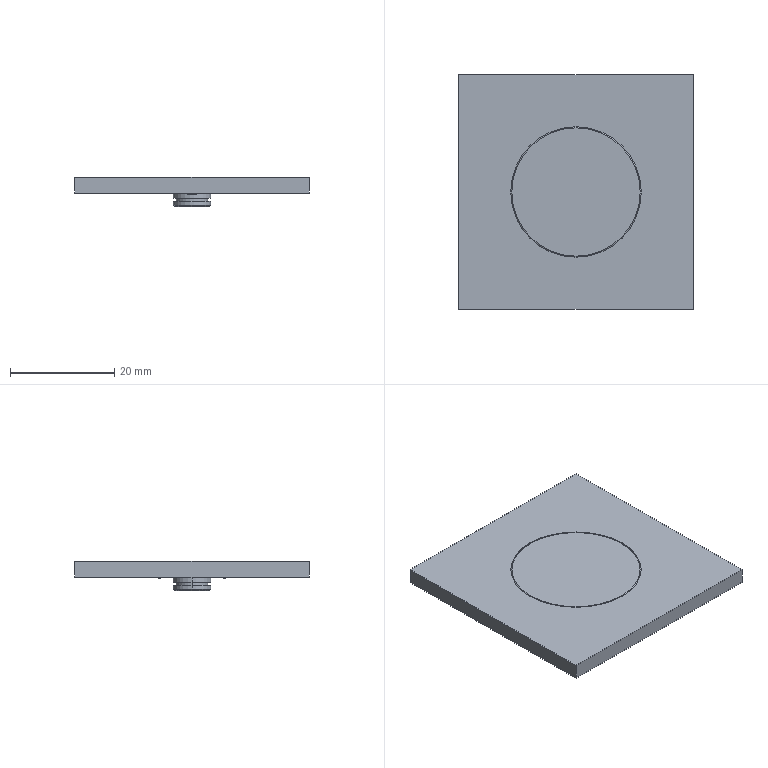Part | 2 solids | 44 faces | box 45 x 45 x 5.6 mm | volume 5766 mm3 | plane 21 | cylinder 9 | cone 8 | spline 4 | torus 2 | commonest cylinder face diameters 7.2 x4 25 x3 6 x2
STEP:
#1=CARTESIAN_POINT('',(-22.5,22.5,0.));
#2=VERTEX_POINT('',#1);
#3=CARTESIAN_POINT('',(-22.5,-22.5,0.));
#4=VERTEX_POINT('',#3);
#5=CARTESIAN_POINT('',(-22.5,22.5,0.));
#6=DIRECTION('',(0.,-1.,0.));
#7=VECTOR('',#6,1000.);
#8=LINE('',#5,#7);
#9=EDGE_CURVE('',#2,#4,#8,.T.);
#10=ORIENTED_EDGE('',*,*,#9,.F.);
#11=CARTESIAN_POINT('',(-22.5,22.5,-3.));
#12=VERTEX_POINT('',#11);
#13=CARTESIAN_POINT('',(-22.5,22.5,-3.));
#14=DIRECTION('',(0.,0.,1.));
#15=VECTOR('',#14,1000.);
#16=LINE('',#13,#15);
#17=EDGE_CURVE('',#12,#2,#16,.T.);
#18=ORIENTED_EDGE('',*,*,#17,.F.);
#19=CARTESIAN_POINT('',(-22.5,-22.5,-3.));
#20=VERTEX_POINT('',#19);
#21=CARTESIAN_POINT('',(-22.5,22.5,-3.));
#22=DIRECTION('',(0.,-1.,0.));
#23=VECTOR('',#22,1000.);
#24=LINE('',#21,#23);
#25=EDGE_CURVE('',#12,#20,#24,.T.);
#26=ORIENTED_EDGE('',*,*,#25,.T.);
#27=CARTESIAN_POINT('',(-22.5,-22.5,-3.));
#28=DIRECTION('',(0.,0.,1.));
#29=VECTOR('',#28,1000.);
#30=LINE('',#27,#29);
#31=EDGE_CURVE('',#20,#4,#30,.T.);
#32=ORIENTED_EDGE('',*,*,#31,.T.);
#33=EDGE_LOOP('',(#10,#18,#26,#32));
#34=FACE_BOUND('',#33,.T.);
#35=CARTESIAN_POINT('',(-22.5,22.5,-3.));
#36=DIRECTION('',(-1.,0.,0.));
#37=DIRECTION('',(0.,0.,1.));
#38=AXIS2_PLACEMENT_3D('',#35,#36,#37);
#39=PLANE('',#38);
#40=ADVANCED_FACE('',(#34),#39,.T.);
#41=CARTESIAN_POINT('',(22.5,-22.5,0.));
#42=VERTEX_POINT('',#41);
#43=CARTESIAN_POINT('',(-22.5,-22.5,0.));
#44=DIRECTION('',(1.,0.,0.));
#45=VECTOR('',#44,1000.);
#46=LINE('',#43,#45);
#47=EDGE_CURVE('',#4,#42,#46,.T.);
#48=ORIENTED_EDGE('',*,*,#47,.F.);
#49=ORIENTED_EDGE('',*,*,#31,.F.);
#50=CARTESIAN_POINT('',(22.5,-22.5,-3.));
#51=VERTEX_POINT('',#50);
#52=CARTESIAN_POINT('',(-22.5,-22.5,-3.));
#53=DIRECTION('',(1.,0.,0.));
#54=VECTOR('',#53,1000.);
#55=LINE('',#52,#54);
#56=EDGE_CURVE('',#20,#51,#55,.T.);
#57=ORIENTED_EDGE('',*,*,#56,.T.);
#58=CARTESIAN_POINT('',(22.5,-22.5,-3.));
#59=DIRECTION('',(0.,0.,1.));
#60=VECTOR('',#59,1000.);
#61=LINE('',#58,#60);
#62=EDGE_CURVE('',#51,#42,#61,.T.);
#63=ORIENTED_EDGE('',*,*,#62,.T.);
#64=EDGE_LOOP('',(#48,#49,#57,#63));
#65=FACE_BOUND('',#64,.T.);
#66=CARTESIAN_POINT('',(-22.5,-22.5,-3.));
#67=DIRECTION('',(0.,-1.,0.));
#68=DIRECTION('',(1.,0.,0.));
#69=AXIS2_PLACEMENT_3D('',#66,#67,#68);
#70=PLANE('',#69);
#71=ADVANCED_FACE('',(#65),#70,.T.);
#72=CARTESIAN_POINT('',(22.5,22.5,0.));
#73=VERTEX_POINT('',#72);
#74=CARTESIAN_POINT('',(22.5,-22.5,0.));
#75=DIRECTION('',(0.,1.,0.));
#76=VECTOR('',#75,1000.);
#77=LINE('',#74,#76);
#78=EDGE_CURVE('',#42,#73,#77,.T.);
#79=ORIENTED_EDGE('',*,*,#78,.F.);
#80=ORIENTED_EDGE('',*,*,#62,.F.);
#81=CARTESIAN_POINT('',(22.5,22.5,-3.));
#82=VERTEX_POINT('',#81);
#83=CARTESIAN_POINT('',(22.5,-22.5,-3.));
#84=DIRECTION('',(0.,1.,0.));
#85=VECTOR('',#84,1000.);
#86=LINE('',#83,#85);
#87=EDGE_CURVE('',#51,#82,#86,.T.);
#88=ORIENTED_EDGE('',*,*,#87,.T.);
#89=CARTESIAN_POINT('',(22.5,22.5,-3.));
#90=DIRECTION('',(0.,0.,1.));
#91=VECTOR('',#90,1000.);
#92=LINE('',#89,#91);
#93=EDGE_CURVE('',#82,#73,#92,.T.);
#94=ORIENTED_EDGE('',*,*,#93,.T.);
#95=EDGE_LOOP('',(#79,#80,#88,#94));
#96=FACE_BOUND('',#95,.T.);
#97=CARTESIAN_POINT('',(22.5,-22.5,-3.));
#98=DIRECTION('',(1.,0.,0.));
#99=DIRECTION('',(0.,1.,0.));
#100=AXIS2_PLACEMENT_3D('',#97,#98,#99);
#101=PLANE('',#100);
#102=ADVANCED_FACE('',(#96),#101,.T.);
#103=CARTESIAN_POINT('',(22.5,22.5,0.));
#104=DIRECTION('',(-1.,0.,0.));
#105=VECTOR('',#104,1000.);
#106=LINE('',#103,#105);
#107=EDGE_CURVE('',#73,#2,#106,.T.);
#108=ORIENTED_EDGE('',*,*,#107,.F.);
#109=ORIENTED_EDGE('',*,*,#93,.F.);
#110=CARTESIAN_POINT('',(22.5,22.5,-3.));
#111=DIRECTION('',(-1.,0.,0.));
#112=VECTOR('',#111,1000.);
#113=LINE('',#110,#112);
#114=EDGE_CURVE('',#82,#12,#113,.T.);
#115=ORIENTED_EDGE('',*,*,#114,.T.);
#116=ORIENTED_EDGE('',*,*,#17,.T.);
#117=EDGE_LOOP('',(#108,#109,#115,#116));
#118=FACE_BOUND('',#117,.T.);
#119=CARTESIAN_POINT('',(22.5,22.5,-3.));
#120=DIRECTION('',(0.,1.,0.));
#121=DIRECTION('',(-1.,0.,0.));
#122=AXIS2_PLACEMENT_3D('',#119,#120,#121);
#123=PLANE('',#122);
#124=ADVANCED_FACE('',(#118),#123,.T.);
#125=CARTESIAN_POINT('',(12.5,0.,-3.));
#126=VERTEX_POINT('',#125);
#127=CARTESIAN_POINT('',(0.,0.,-3.));
#128=DIRECTION('',(0.,0.,1.));
#129=DIRECTION('',(1.,0.,0.));
#130=AXIS2_PLACEMENT_3D('',#127,#128,#129);
#131=CIRCLE('',#130,12.5);
#132=EDGE_CURVE('',#126,#126,#131,.T.);
#133=ORIENTED_EDGE('',*,*,#132,.F.);
#134=EDGE_LOOP('',(#133));
#135=FACE_BOUND('',#134,.T.);
#136=CARTESIAN_POINT('',(12.5,0.,0.));
#137=VERTEX_POINT('',#136);
#138=CARTESIAN_POINT('',(0.,0.,0.));
#139=DIRECTION('',(0.,0.,1.));
#140=DIRECTION('',(1.,0.,0.));
#141=AXIS2_PLACEMENT_3D('',#138,#139,#140);
#142=CIRCLE('',#141,12.5);
#143=EDGE_CURVE('',#137,#137,#142,.T.);
#144=ORIENTED_EDGE('',*,*,#143,.T.);
#145=EDGE_LOOP('',(#144));
#146=FACE_BOUND('',#145,.T.);
#147=CARTESIAN_POINT('',(0.,0.,-3.));
#148=DIRECTION('',(0.,0.,1.));
#149=DIRECTION('',(1.,0.,0.));
#150=AXIS2_PLACEMENT_3D('',#147,#148,#149);
#151=CYLINDRICAL_SURFACE('',#150,12.5);
#152=ADVANCED_FACE('',(#135,#146),#151,.F.);
#153=ORIENTED_EDGE('',*,*,#25,.F.);
#154=ORIENTED_EDGE('',*,*,#114,.F.);
#155=ORIENTED_EDGE('',*,*,#87,.F.);
#156=ORIENTED_EDGE('',*,*,#56,.F.);
#157=EDGE_LOOP('',(#153,#154,#155,#156));
#158=FACE_BOUND('',#157,.T.);
#159=ORIENTED_EDGE('',*,*,#132,.T.);
#160=EDGE_LOOP('',(#159));
#161=FACE_BOUND('',#160,.T.);
#162=CARTESIAN_POINT('',(0.,0.,-3.));
#163=DIRECTION('',(0.,0.,1.));
#164=DIRECTION('',(1.,0.,0.));
#165=AXIS2_PLACEMENT_3D('',#162,#163,#164);
#166=PLANE('',#165);
#167=ADVANCED_FACE('',(#158,#161),#166,.F.);
#168=ORIENTED_EDGE('',*,*,#9,.T.);
#169=ORIENTED_EDGE('',*,*,#47,.T.);
#170=ORIENTED_EDGE('',*,*,#78,.T.);
#171=ORIENTED_EDGE('',*,*,#107,.T.);
#172=EDGE_LOOP('',(#168,#169,#170,#171));
#173=FACE_BOUND('',#172,.T.);
#174=ORIENTED_EDGE('',*,*,#143,.F.);
#175=EDGE_LOOP('',(#174));
#176=FACE_BOUND('',#175,.T.);
#177=CARTESIAN_POINT('',(0.,0.,0.));
#178=DIRECTION('',(0.,0.,1.));
#179=DIRECTION('',(1.,0.,0.));
#180=AXIS2_PLACEMENT_3D('',#177,#178,#179);
#181=PLANE('',#180);
#182=ADVANCED_FACE('',(#173,#176),#181,.T.);
#183=CLOSED_SHELL('',(#40,#71,#102,#124,#152,#167,#182));
#184=MANIFOLD_SOLID_BREP('',#183);
#185=CARTESIAN_POINT('',(12.2,0.,-2.1));
#186=VERTEX_POINT('',#185);
#187=CARTESIAN_POINT('',(-12.2,0.,-2.1));
#188=VERTEX_POINT('',#187);
#189=CARTESIAN_POINT('',(0.,0.,-2.1));
#190=DIRECTION('',(0.,0.,-1.));
#191=DIRECTION('',(1.,0.,0.));
#192=AXIS2_PLACEMENT_3D('',#189,#190,#191);
#193=CIRCLE('',#192,12.2);
#194=EDGE_CURVE('',#186,#188,#193,.T.);
#195=ORIENTED_EDGE('',*,*,#194,.T.);
#196=CARTESIAN_POINT('',(0.,0.,-2.1));
#197=DIRECTION('',(0.,0.,-1.));
#198=DIRECTION('',(-1.,0.,0.));
#199=AXIS2_PLACEMENT_3D('',#196,#197,#198);
#200=CIRCLE('',#199,12.2);
#201=EDGE_CURVE('',#188,#186,#200,.T.);
#202=ORIENTED_EDGE('',*,*,#201,.T.);
#203=EDGE_LOOP('',(#195,#202));
#204=FACE_BOUND('',#203,.T.);
#205=CARTESIAN_POINT('',(-0.55,6.621,-2.1));
#206=VERTEX_POINT('',#205);
#207=CARTESIAN_POINT('',(-0.55,5.779,-2.1));
#208=VERTEX_POINT('',#207);
#209=CARTESIAN_POINT('',(-0.55,6.2,-2.1));
#210=DIRECTION('',(0.,0.,1.));
#211=DIRECTION('',(0.,1.,0.));
#212=AXIS2_PLACEMENT_3D('',#209,#210,#211);
#213=CIRCLE('',#212,0.4209);
#214=EDGE_CURVE('',#206,#208,#213,.T.);
#215=ORIENTED_EDGE('',*,*,#214,.T.);
#216=CARTESIAN_POINT('',(0.55,5.779,-2.1));
#217=VERTEX_POINT('',#216);
#218=CARTESIAN_POINT('',(-0.55,5.779,-2.1));
#219=DIRECTION('',(1.,0.,0.));
#220=VECTOR('',#219,1000.);
#221=LINE('',#218,#220);
#222=EDGE_CURVE('',#208,#217,#221,.T.);
#223=ORIENTED_EDGE('',*,*,#222,.T.);
#224=CARTESIAN_POINT('',(0.55,6.621,-2.1));
#225=VERTEX_POINT('',#224);
#226=CARTESIAN_POINT('',(0.55,6.2,-2.1));
#227=DIRECTION('',(0.,0.,1.));
#228=DIRECTION('',(0.,-1.,0.));
#229=AXIS2_PLACEMENT_3D('',#226,#227,#228);
#230=CIRCLE('',#229,0.4209);
#231=EDGE_CURVE('',#217,#225,#230,.T.);
#232=ORIENTED_EDGE('',*,*,#231,.T.);
#233=CARTESIAN_POINT('',(0.55,6.621,-2.1));
#234=DIRECTION('',(-1.,0.,0.));
#235=VECTOR('',#234,1000.);
#236=LINE('',#233,#235);
#237=EDGE_CURVE('',#225,#206,#236,.T.);
#238=ORIENTED_EDGE('',*,*,#237,.T.);
#239=EDGE_LOOP('',(#215,#223,#232,#238));
#240=FACE_BOUND('',#239,.T.);
#241=CARTESIAN_POINT('',(0.55,-6.621,-2.1));
#242=VERTEX_POINT('',#241);
#243=CARTESIAN_POINT('',(0.55,-5.779,-2.1));
#244=VERTEX_POINT('',#243);
#245=CARTESIAN_POINT('',(0.55,-6.2,-2.1));
#246=DIRECTION('',(0.,0.,1.));
#247=DIRECTION('',(0.,-1.,0.));
#248=AXIS2_PLACEMENT_3D('',#245,#246,#247);
#249=CIRCLE('',#248,0.4209);
#250=EDGE_CURVE('',#242,#244,#249,.T.);
#251=ORIENTED_EDGE('',*,*,#250,.T.);
#252=CARTESIAN_POINT('',(-0.55,-5.779,-2.1));
#253=VERTEX_POINT('',#252);
#254=CARTESIAN_POINT('',(0.55,-5.779,-2.1));
#255=DIRECTION('',(-1.,0.,0.));
#256=VECTOR('',#255,1000.);
#257=LINE('',#254,#256);
#258=EDGE_CURVE('',#244,#253,#257,.T.);
#259=ORIENTED_EDGE('',*,*,#258,.T.);
#260=CARTESIAN_POINT('',(-0.55,-6.621,-2.1));
#261=VERTEX_POINT('',#260);
#262=CARTESIAN_POINT('',(-0.55,-6.2,-2.1));
#263=DIRECTION('',(0.,0.,1.));
#264=DIRECTION('',(0.,1.,0.));
#265=AXIS2_PLACEMENT_3D('',#262,#263,#264);
#266=CIRCLE('',#265,0.4209);
#267=EDGE_CURVE('',#253,#261,#266,.T.);
#268=ORIENTED_EDGE('',*,*,#267,.T.);
#269=CARTESIAN_POINT('',(-0.55,-6.621,-2.1));
#270=DIRECTION('',(1.,0.,0.));
#271=VECTOR('',#270,1000.);
#272=LINE('',#269,#271);
#273=EDGE_CURVE('',#261,#242,#272,.T.);
#274=ORIENTED_EDGE('',*,*,#273,.T.);
#275=EDGE_LOOP('',(#251,#259,#268,#274));
#276=FACE_BOUND('',#275,.T.);
#277=CARTESIAN_POINT('',(-3.6,0.,-2.1));
#278=VERTEX_POINT('',#277);
#279=CARTESIAN_POINT('',(3.6,0.,-2.1));
#280=VERTEX_POINT('',#279);
#281=CARTESIAN_POINT('',(0.,0.,-2.1));
#282=DIRECTION('',(0.,0.,1.));
#283=DIRECTION('',(-1.,0.,0.));
#284=AXIS2_PLACEMENT_3D('',#281,#282,#283);
#285=CIRCLE('',#284,3.6);
#286=EDGE_CURVE('',#278,#280,#285,.T.);
#287=ORIENTED_EDGE('',*,*,#286,.T.);
#288=CARTESIAN_POINT('',(0.,0.,-2.1));
#289=DIRECTION('',(0.,0.,1.));
#290=DIRECTION('',(1.,0.,0.));
#291=AXIS2_PLACEMENT_3D('',#288,#289,#290);
#292=CIRCLE('',#291,3.6);
#293=EDGE_CURVE('',#280,#278,#292,.T.);
#294=ORIENTED_EDGE('',*,*,#293,.T.);
#295=EDGE_LOOP('',(#287,#294));
#296=FACE_BOUND('',#295,.T.);
#297=CARTESIAN_POINT('',(0.,0.,-2.1));
#298=DIRECTION('',(0.,0.,1.));
#299=DIRECTION('',(-1.,0.,0.));
#300=AXIS2_PLACEMENT_3D('',#297,#298,#299);
#301=PLANE('',#300);
#302=ADVANCED_FACE('',(#204,#240,#276,#296),#301,.F.);
#303=CARTESIAN_POINT('',(-3.6,0.,-4.));
#304=VERTEX_POINT('',#303);
#305=CARTESIAN_POINT('',(-3.6,0.,-2.1));
#306=DIRECTION('',(0.,0.,-1.));
#307=VECTOR('',#306,1000.);
#308=LINE('',#305,#307);
#309=EDGE_CURVE('',#278,#304,#308,.T.);
#310=ORIENTED_EDGE('',*,*,#309,.F.);
#311=ORIENTED_EDGE('',*,*,#293,.F.);
#312=CARTESIAN_POINT('',(3.6,0.,-4.));
#313=VERTEX_POINT('',#312);
#314=CARTESIAN_POINT('',(3.6,0.,-2.1));
#315=DIRECTION('',(0.,0.,-1.));
#316=VECTOR('',#315,1000.);
#317=LINE('',#314,#316);
#318=EDGE_CURVE('',#280,#313,#317,.T.);
#319=ORIENTED_EDGE('',*,*,#318,.T.);
#320=CARTESIAN_POINT('',(0.,0.,-4.));
#321=DIRECTION('',(0.,0.,1.));
#322=DIRECTION('',(1.,0.,0.));
#323=AXIS2_PLACEMENT_3D('',#320,#321,#322);
#324=CIRCLE('',#323,3.6);
#325=EDGE_CURVE('',#313,#304,#324,.T.);
#326=ORIENTED_EDGE('',*,*,#325,.T.);
#327=EDGE_LOOP('',(#310,#311,#319,#326));
#328=FACE_BOUND('',#327,.T.);
#329=CARTESIAN_POINT('',(0.,0.,-2.1));
#330=DIRECTION('',(0.,0.,1.));
#331=DIRECTION('',(-1.,0.,0.));
#332=AXIS2_PLACEMENT_3D('',#329,#330,#331);
#333=CYLINDRICAL_SURFACE('',#332,3.6);
#334=ADVANCED_FACE('',(#328),#333,.T.);
#335=CARTESIAN_POINT('',(-3.6,0.,-4.6));
#336=VERTEX_POINT('',#335);
#337=CARTESIAN_POINT('',(-3.6,0.,-5.3));
#338=VERTEX_POINT('',#337);
#339=CARTESIAN_POINT('',(-3.6,0.,-4.6));
#340=DIRECTION('',(0.,-0.000000001,-1.));
#341=VECTOR('',#340,1000.);
#342=LINE('',#339,#341);
#343=EDGE_CURVE('',#336,#338,#342,.T.);
#344=ORIENTED_EDGE('',*,*,#343,.F.);
#345=CARTESIAN_POINT('',(3.6,0.,-4.6));
#346=VERTEX_POINT('',#345);
#347=CARTESIAN_POINT('',(0.,0.,-4.6));
#348=DIRECTION('',(0.,0.,1.));
#349=DIRECTION('',(1.,0.,0.));
#350=AXIS2_PLACEMENT_3D('',#347,#348,#349);
#351=CIRCLE('',#350,3.6);
#352=EDGE_CURVE('',#346,#336,#351,.T.);
#353=ORIENTED_EDGE('',*,*,#352,.F.);
#354=CARTESIAN_POINT('',(3.6,0.,-5.3));
#355=VERTEX_POINT('',#354);
#356=CARTESIAN_POINT('',(3.6,0.,-4.6));
#357=DIRECTION('',(0.,0.000000001,-1.));
#358=VECTOR('',#357,1000.);
#359=LINE('',#356,#358);
#360=EDGE_CURVE('',#346,#355,#359,.T.);
#361=ORIENTED_EDGE('',*,*,#360,.T.);
#362=CARTESIAN_POINT('',(0.,0.,-5.3));
#363=DIRECTION('',(0.,0.,-1.));
#364=DIRECTION('',(-1.,0.,0.));
#365=AXIS2_PLACEMENT_3D('',#362,#363,#364);
#366=CIRCLE('',#365,3.6);
#367=EDGE_CURVE('',#338,#355,#366,.T.);
#368=ORIENTED_EDGE('',*,*,#367,.F.);
#369=EDGE_LOOP('',(#344,#353,#361,#368));
#370=FACE_BOUND('',#369,.T.);
#371=CARTESIAN_POINT('',(0.,0.,-2.1));
#372=DIRECTION('',(0.,0.,1.));
#373=DIRECTION('',(-1.,0.,0.));
#374=AXIS2_PLACEMENT_3D('',#371,#372,#373);
#375=CYLINDRICAL_SURFACE('',#374,3.6);
#376=ADVANCED_FACE('',(#370),#375,.T.);
#377=CARTESIAN_POINT('',(0.,0.,-4.));
#378=DIRECTION('',(0.,0.,1.));
#379=DIRECTION('',(-1.,0.,0.));
#380=AXIS2_PLACEMENT_3D('',#377,#378,#379);
#381=CIRCLE('',#380,3.6);
#382=EDGE_CURVE('',#304,#313,#381,.T.);
#383=ORIENTED_EDGE('',*,*,#382,.F.);
#384=ORIENTED_EDGE('',*,*,#325,.F.);
#385=EDGE_LOOP('',(#383,#384));
#386=FACE_BOUND('',#385,.T.);
#387=CARTESIAN_POINT('',(3.,0.,-4.));
#388=VERTEX_POINT('',#387);
#389=CARTESIAN_POINT('',(-3.,0.,-4.));
#390=VERTEX_POINT('',#389);
#391=CARTESIAN_POINT('',(0.,0.,-4.));
#392=DIRECTION('',(0.,0.,1.));
#393=DIRECTION('',(1.,0.,0.));
#394=AXIS2_PLACEMENT_3D('',#391,#392,#393);
#395=CIRCLE('',#394,3.);
#396=EDGE_CURVE('',#388,#390,#395,.T.);
#397=ORIENTED_EDGE('',*,*,#396,.T.);
#398=CARTESIAN_POINT('',(0.,0.,-4.));
#399=DIRECTION('',(0.,0.,-1.));
#400=DIRECTION('',(1.,0.,0.));
#401=AXIS2_PLACEMENT_3D('',#398,#399,#400);
#402=CIRCLE('',#401,3.);
#403=EDGE_CURVE('',#388,#390,#402,.T.);
#404=ORIENTED_EDGE('',*,*,#403,.F.);
#405=EDGE_LOOP('',(#397,#404));
#406=FACE_BOUND('',#405,.T.);
#407=CARTESIAN_POINT('',(0.,0.,-4.));
#408=DIRECTION('',(0.,0.,-1.));
#409=DIRECTION('',(1.,0.,0.));
#410=AXIS2_PLACEMENT_3D('',#407,#408,#409);
#411=PLANE('',#410);
#412=ADVANCED_FACE('',(#386,#406),#411,.T.);
#413=ORIENTED_EDGE('',*,*,#403,.T.);
#414=CARTESIAN_POINT('',(-3.,0.,-4.6));
#415=VERTEX_POINT('',#414);
#416=CARTESIAN_POINT('',(-3.,0.,-4.));
#417=DIRECTION('',(0.,0.,-1.));
#418=VECTOR('',#417,1000.);
#419=LINE('',#416,#418);
#420=EDGE_CURVE('',#390,#415,#419,.T.);
#421=ORIENTED_EDGE('',*,*,#420,.T.);
#422=CARTESIAN_POINT('',(3.,0.,-4.6));
#423=VERTEX_POINT('',#422);
#424=CARTESIAN_POINT('',(0.,0.,-4.6));
#425=DIRECTION('',(0.,0.,-1.));
#426=DIRECTION('',(1.,0.,0.));
#427=AXIS2_PLACEMENT_3D('',#424,#425,#426);
#428=CIRCLE('',#427,3.);
#429=EDGE_CURVE('',#423,#415,#428,.T.);
#430=ORIENTED_EDGE('',*,*,#429,.F.);
#431=CARTESIAN_POINT('',(3.,0.,-4.));
#432=DIRECTION('',(0.,0.,-1.));
#433=VECTOR('',#432,1000.);
#434=LINE('',#431,#433);
#435=EDGE_CURVE('',#388,#423,#434,.T.);
#436=ORIENTED_EDGE('',*,*,#435,.F.);
#437=EDGE_LOOP('',(#413,#421,#430,#436));
#438=FACE_BOUND('',#437,.T.);
#439=CARTESIAN_POINT('',(0.,0.,-3.97));
#440=DIRECTION('',(0.,0.,-1.));
#441=DIRECTION('',(1.,0.,0.));
#442=AXIS2_PLACEMENT_3D('',#439,#440,#441);
#443=CYLINDRICAL_SURFACE('',#442,3.);
#444=ADVANCED_FACE('',(#438),#443,.T.);
#445=CARTESIAN_POINT('',(0.,0.,-4.6));
#446=DIRECTION('',(0.,0.,1.));
#447=DIRECTION('',(1.,0.,0.));
#448=AXIS2_PLACEMENT_3D('',#445,#446,#447);
#449=CIRCLE('',#448,3.);
#450=EDGE_CURVE('',#423,#415,#449,.T.);
#451=ORIENTED_EDGE('',*,*,#450,.T.);
#452=ORIENTED_EDGE('',*,*,#420,.F.);
#453=ORIENTED_EDGE('',*,*,#396,.F.);
#454=ORIENTED_EDGE('',*,*,#435,.T.);
#455=EDGE_LOOP('',(#451,#452,#453,#454));
#456=FACE_BOUND('',#455,.T.);
#457=CARTESIAN_POINT('',(0.,0.,-3.97));
#458=DIRECTION('',(0.,0.,-1.));
#459=DIRECTION('',(1.,0.,0.));
#460=AXIS2_PLACEMENT_3D('',#457,#458,#459);
#461=CYLINDRICAL_SURFACE('',#460,3.);
#462=ADVANCED_FACE('',(#456),#461,.T.);
#463=CARTESIAN_POINT('',(0.,0.,-4.6));
#464=DIRECTION('',(0.,0.,1.));
#465=DIRECTION('',(-1.,0.,0.));
#466=AXIS2_PLACEMENT_3D('',#463,#464,#465);
#467=CIRCLE('',#466,3.6);
#468=EDGE_CURVE('',#336,#346,#467,.T.);
#469=ORIENTED_EDGE('',*,*,#468,.T.);
#470=ORIENTED_EDGE('',*,*,#352,.T.);
#471=EDGE_LOOP('',(#469,#470));
#472=FACE_BOUND('',#471,.T.);
#473=ORIENTED_EDGE('',*,*,#429,.T.);
#474=ORIENTED_EDGE('',*,*,#450,.F.);
#475=EDGE_LOOP('',(#473,#474));
#476=FACE_BOUND('',#475,.T.);
#477=CARTESIAN_POINT('',(0.,0.,-4.6));
#478=DIRECTION('',(0.,0.,-1.));
#479=DIRECTION('',(1.,0.,0.));
#480=AXIS2_PLACEMENT_3D('',#477,#478,#479);
#481=PLANE('',#480);
#482=ADVANCED_FACE('',(#472,#476),#481,.F.);
#483=ORIENTED_EDGE('',*,*,#318,.F.);
#484=ORIENTED_EDGE('',*,*,#286,.F.);
#485=ORIENTED_EDGE('',*,*,#309,.T.);
#486=ORIENTED_EDGE('',*,*,#382,.T.);
#487=EDGE_LOOP('',(#483,#484,#485,#486));
#488=FACE_BOUND('',#487,.T.);
#489=CARTESIAN_POINT('',(0.,0.,-2.1));
#490=DIRECTION('',(0.,0.,1.));
#491=DIRECTION('',(-1.,0.,0.));
#492=AXIS2_PLACEMENT_3D('',#489,#490,#491);
#493=CYLINDRICAL_SURFACE('',#492,3.6);
#494=ADVANCED_FACE('',(#488),#493,.T.);
#495=ORIENTED_EDGE('',*,*,#360,.F.);
#496=ORIENTED_EDGE('',*,*,#468,.F.);
#497=ORIENTED_EDGE('',*,*,#343,.T.);
#498=CARTESIAN_POINT('',(0.,0.,-5.3));
#499=DIRECTION('',(0.,0.,-1.));
#500=DIRECTION('',(1.,0.,0.));
#501=AXIS2_PLACEMENT_3D('',#498,#499,#500);
#502=CIRCLE('',#501,3.6);
#503=EDGE_CURVE('',#355,#338,#502,.T.);
#504=ORIENTED_EDGE('',*,*,#503,.F.);
#505=EDGE_LOOP('',(#495,#496,#497,#504));
#506=FACE_BOUND('',#505,.T.);
#507=CARTESIAN_POINT('',(0.,0.,-2.1));
#508=DIRECTION('',(0.,0.,1.));
#509=DIRECTION('',(-1.,0.,0.));
#510=AXIS2_PLACEMENT_3D('',#507,#508,#509);
#511=CYLINDRICAL_SURFACE('',#510,3.6);
#512=ADVANCED_FACE('',(#506),#511,.T.);
#513=CARTESIAN_POINT('',(3.3,0.,-5.6));
#514=VERTEX_POINT('',#513);
#515=CARTESIAN_POINT('',(3.3,0.000000001,-5.6));
#516=DIRECTION('',(0.7071,0.,0.7071));
#517=VECTOR('',#516,1000.);
#518=LINE('',#515,#517);
#519=EDGE_CURVE('',#514,#355,#518,.T.);
#520=ORIENTED_EDGE('',*,*,#519,.T.);
#521=ORIENTED_EDGE('',*,*,#503,.T.);
#522=CARTESIAN_POINT('',(-3.3,0.,-5.6));
#523=VERTEX_POINT('',#522);
#524=CARTESIAN_POINT('',(-3.3,-0.000000001,-5.6));
#525=DIRECTION('',(-0.7071,0.,0.7071));
#526=VECTOR('',#525,1000.);
#527=LINE('',#524,#526);
#528=EDGE_CURVE('',#523,#338,#527,.T.);
#529=ORIENTED_EDGE('',*,*,#528,.F.);
#530=CARTESIAN_POINT('',(0.,0.,-5.6));
#531=DIRECTION('',(0.,0.,-1.));
#532=DIRECTION('',(1.,0.,0.));
#533=AXIS2_PLACEMENT_3D('',#530,#531,#532);
#534=CIRCLE('',#533,3.3);
#535=EDGE_CURVE('',#514,#523,#534,.T.);
#536=ORIENTED_EDGE('',*,*,#535,.F.);
#537=EDGE_LOOP('',(#520,#521,#529,#536));
#538=FACE_BOUND('',#537,.T.);
#539=CARTESIAN_POINT('',(0.,0.,-5.45));
#540=DIRECTION('',(0.,0.,1.));
#541=DIRECTION('',(0.,-1.,0.));
#542=AXIS2_PLACEMENT_3D('',#539,#540,#541);
#543=CONICAL_SURFACE('',#542,3.45,0.7854);
#544=ADVANCED_FACE('',(#538),#543,.T.);
#545=ORIENTED_EDGE('',*,*,#535,.T.);
#546=CARTESIAN_POINT('',(0.,0.,-5.6));
#547=DIRECTION('',(0.,0.,-1.));
#548=DIRECTION('',(-1.,0.,0.));
#549=AXIS2_PLACEMENT_3D('',#546,#547,#548);
#550=CIRCLE('',#549,3.3);
#551=EDGE_CURVE('',#523,#514,#550,.T.);
#552=ORIENTED_EDGE('',*,*,#551,.T.);
#553=EDGE_LOOP('',(#545,#552));
#554=FACE_BOUND('',#553,.T.);
#555=CARTESIAN_POINT('',(0.,0.,-5.6));
#556=DIRECTION('',(0.,0.,1.));
#557=DIRECTION('',(-1.,0.,0.));
#558=AXIS2_PLACEMENT_3D('',#555,#556,#557);
#559=PLANE('',#558);
#560=ADVANCED_FACE('',(#554),#559,.F.);
#561=ORIENTED_EDGE('',*,*,#528,.T.);
#562=ORIENTED_EDGE('',*,*,#367,.T.);
#563=ORIENTED_EDGE('',*,*,#519,.F.);
#564=ORIENTED_EDGE('',*,*,#551,.F.);
#565=EDGE_LOOP('',(#561,#562,#563,#564));
#566=FACE_BOUND('',#565,.T.);
#567=CARTESIAN_POINT('',(0.,0.,-5.45));
#568=DIRECTION('',(0.,0.,1.));
#569=DIRECTION('',(0.,-1.,0.));
#570=AXIS2_PLACEMENT_3D('',#567,#568,#569);
#571=CONICAL_SURFACE('',#570,3.45,0.7854);
#572=ADVANCED_FACE('',(#566),#571,.T.);
#573=CARTESIAN_POINT('',(-0.55,6.603,-3.1));
#574=VERTEX_POINT('',#573);
#575=CARTESIAN_POINT('',(-0.55,6.621,-2.1));
#576=CARTESIAN_POINT('',(-0.55,6.615,-2.433));
#577=CARTESIAN_POINT('',(-0.55,6.609,-2.767));
#578=CARTESIAN_POINT('',(-0.55,6.603,-3.1));
#579=B_SPLINE_CURVE_WITH_KNOTS('',3,(#575,#576,#577,#578),.UNSPECIFIED.,.F.,.F.,(4,4),(0.,1.),.PIECEWISE_BEZIER_KNOTS.);
#580=EDGE_CURVE('',#206,#574,#579,.T.);
#581=ORIENTED_EDGE('',*,*,#580,.F.);
#582=ORIENTED_EDGE('',*,*,#237,.F.);
#583=CARTESIAN_POINT('',(0.55,6.603,-3.1));
#584=VERTEX_POINT('',#583);
#585=CARTESIAN_POINT('',(0.55,6.603,-3.1));
#586=CARTESIAN_POINT('',(0.55,6.609,-2.767));
#587=CARTESIAN_POINT('',(0.55,6.615,-2.433));
#588=CARTESIAN_POINT('',(0.55,6.621,-2.1));
#589=B_SPLINE_CURVE_WITH_KNOTS('',3,(#585,#586,#587,#588),.UNSPECIFIED.,.F.,.F.,(4,4),(0.,1.),.PIECEWISE_BEZIER_KNOTS.);
#590=EDGE_CURVE('',#584,#225,#589,.T.);
#591=ORIENTED_EDGE('',*,*,#590,.F.);
#592=CARTESIAN_POINT('',(-0.55,6.603,-3.1));
#593=DIRECTION('',(1.,-0.000002525,0.000002569));
#594=VECTOR('',#593,1000.);
#595=LINE('',#592,#594);
#596=EDGE_CURVE('',#574,#584,#595,.T.);
#597=ORIENTED_EDGE('',*,*,#596,.F.);
#598=EDGE_LOOP('',(#581,#582,#591,#597));
#599=FACE_BOUND('',#598,.T.);
#600=CARTESIAN_POINT('',(2.31,6.6,-3.3));
#601=DIRECTION('',(0.,0.9998,-0.01745));
#602=DIRECTION('',(-1.,0.,0.));
#603=AXIS2_PLACEMENT_3D('',#600,#601,#602);
#604=PLANE('',#603);
#605=ADVANCED_FACE('',(#599),#604,.T.);
#606=CARTESIAN_POINT('',(0.55,6.4,-3.3));
#607=VERTEX_POINT('',#606);
#608=CARTESIAN_POINT('',(0.55,6.4,-3.3));
#609=DIRECTION('',(0.,0.7132,0.7009));
#610=VECTOR('',#609,1000.);
#611=LINE('',#608,#610);
#612=EDGE_CURVE('',#607,#584,#611,.T.);
#613=ORIENTED_EDGE('',*,*,#612,.F.);
#614=CARTESIAN_POINT('',(-0.55,6.4,-3.3));
#615=VERTEX_POINT('',#614);
#616=CARTESIAN_POINT('',(-0.55,6.4,-3.3));
#617=DIRECTION('',(1.,-0.000001669,0.000001698));
#618=VECTOR('',#617,1000.);
#619=LINE('',#616,#618);
#620=EDGE_CURVE('',#615,#607,#619,.T.);
#621=ORIENTED_EDGE('',*,*,#620,.F.);
#622=CARTESIAN_POINT('',(-0.55,6.4,-3.3));
#623=DIRECTION('',(-0.000000001,0.7133,0.7009));
#624=VECTOR('',#623,1000.);
#625=LINE('',#622,#624);
#626=EDGE_CURVE('',#615,#574,#625,.T.);
#627=ORIENTED_EDGE('',*,*,#626,.T.);
#628=ORIENTED_EDGE('',*,*,#596,.T.);
#629=EDGE_LOOP('',(#613,#621,#627,#628));
#630=FACE_BOUND('',#629,.T.);
#631=CARTESIAN_POINT('',(0.,6.502,-3.2));
#632=DIRECTION('',(0.,0.7009,-0.7133));
#633=DIRECTION('',(0.,-0.7133,-0.7009));
#634=AXIS2_PLACEMENT_3D('',#631,#632,#633);
#635=PLANE('',#634);
#636=ADVANCED_FACE('',(#630),#635,.T.);
#637=CARTESIAN_POINT('',(-0.55,6.,-3.3));
#638=VERTEX_POINT('',#637);
#639=CARTESIAN_POINT('',(-0.55,5.797,-3.1));
#640=VERTEX_POINT('',#639);
#641=CARTESIAN_POINT('',(-0.55,5.797,-3.1));
#642=CARTESIAN_POINT('',(-0.55,5.864,-3.167));
#643=CARTESIAN_POINT('',(-0.55,5.932,-3.233));
#644=CARTESIAN_POINT('',(-0.55,6.,-3.3));
#645=B_SPLINE_CURVE_WITH_KNOTS('',3,(#641,#642,#643,#644),.UNSPECIFIED.,.F.,.F.,(4,4),(0.,1.),.UNSPECIFIED.);
#646=EDGE_CURVE('',#638,#640,#645,.F.);
#647=ORIENTED_EDGE('',*,*,#646,.T.);
#648=CARTESIAN_POINT('',(-0.55,5.797,-3.1));
#649=CARTESIAN_POINT('',(-0.7632,5.797,-3.1));
#650=CARTESIAN_POINT('',(-1.144,6.2,-3.1));
#651=CARTESIAN_POINT('',(-0.7632,6.603,-3.1));
#652=CARTESIAN_POINT('',(-0.55,6.603,-3.1));
#653=B_SPLINE_CURVE_WITH_KNOTS('',3,(#648,#649,#650,#651,#652),.UNSPECIFIED.,.F.,.F.,(4,1,4),(0.,0.0006324,0.001265),.UNSPECIFIED.);
#654=EDGE_CURVE('',#640,#574,#653,.T.);
#655=ORIENTED_EDGE('',*,*,#654,.T.);
#656=ORIENTED_EDGE('',*,*,#626,.F.);
#657=CARTESIAN_POINT('',(-0.55,6.,-3.3));
#658=CARTESIAN_POINT('',(-0.6557,6.,-3.3));
#659=CARTESIAN_POINT('',(-0.8443,6.2,-3.3));
#660=CARTESIAN_POINT('',(-0.6557,6.4,-3.3));
#661=CARTESIAN_POINT('',(-0.55,6.4,-3.3));
#662=B_SPLINE_CURVE_WITH_KNOTS('',3,(#657,#658,#659,#660,#661),.UNSPECIFIED.,.F.,.F.,(4,1,4),(0.,0.0003126,0.0006253),.UNSPECIFIED.);
#663=EDGE_CURVE('',#638,#615,#662,.T.);
#664=ORIENTED_EDGE('',*,*,#663,.F.);
#665=EDGE_LOOP('',(#647,#655,#656,#664));
#666=FACE_BOUND('',#665,.T.);
#667=CARTESIAN_POINT('',(-0.55,6.001,-3.301));
#668=CARTESIAN_POINT('',(-0.55,5.933,-3.234));
#669=CARTESIAN_POINT('',(-0.55,5.864,-3.166));
#670=CARTESIAN_POINT('',(-0.55,5.795,-3.099));
#671=CARTESIAN_POINT('',(-0.5614,6.001,-3.301));
#672=CARTESIAN_POINT('',(-0.5654,5.933,-3.234));
#673=CARTESIAN_POINT('',(-0.5693,5.864,-3.166));
#674=CARTESIAN_POINT('',(-0.5732,5.795,-3.099));
#675=CARTESIAN_POINT('',(-0.5917,6.004,-3.301));
#676=CARTESIAN_POINT('',(-0.606,5.936,-3.234));
#677=CARTESIAN_POINT('',(-0.6204,5.868,-3.166));
#678=CARTESIAN_POINT('',(-0.6348,5.801,-3.099));
#679=CARTESIAN_POINT('',(-0.6388,6.019,-3.301));
#680=CARTESIAN_POINT('',(-0.6695,5.957,-3.234));
#681=CARTESIAN_POINT('',(-0.7002,5.894,-3.166));
#682=CARTESIAN_POINT('',(-0.7308,5.832,-3.099));
#683=CARTESIAN_POINT('',(-0.686,6.051,-3.301));
#684=CARTESIAN_POINT('',(-0.733,6.,-3.234));
#685=CARTESIAN_POINT('',(-0.78,5.949,-3.166));
#686=CARTESIAN_POINT('',(-0.8269,5.897,-3.099));
#687=CARTESIAN_POINT('',(-0.7222,6.095,-3.301));
#688=CARTESIAN_POINT('',(-0.7817,6.059,-3.234));
#689=CARTESIAN_POINT('',(-0.8412,6.023,-3.166));
#690=CARTESIAN_POINT('',(-0.9007,5.987,-3.099));
#691=CARTESIAN_POINT('',(-0.7446,6.148,-3.301));
#692=CARTESIAN_POINT('',(-0.8119,6.13,-3.234));
#693=CARTESIAN_POINT('',(-0.8791,6.112,-3.166));
#694=CARTESIAN_POINT('',(-0.9464,6.094,-3.099));
#695=CARTESIAN_POINT('',(-0.7514,6.205,-3.301));
#696=CARTESIAN_POINT('',(-0.821,6.206,-3.234));
#697=CARTESIAN_POINT('',(-0.8905,6.208,-3.166));
#698=CARTESIAN_POINT('',(-0.9601,6.21,-3.099));
#699=CARTESIAN_POINT('',(-0.742,6.261,-3.301));
#700=CARTESIAN_POINT('',(-0.8083,6.282,-3.234));
#701=CARTESIAN_POINT('',(-0.8746,6.303,-3.166));
#702=CARTESIAN_POINT('',(-0.9409,6.324,-3.099));
#703=CARTESIAN_POINT('',(-0.7171,6.313,-3.301));
#704=CARTESIAN_POINT('',(-0.7748,6.351,-3.234));
#705=CARTESIAN_POINT('',(-0.8326,6.39,-3.166));
#706=CARTESIAN_POINT('',(-0.8903,6.429,-3.099));
#707=CARTESIAN_POINT('',(-0.6788,6.355,-3.301));
#708=CARTESIAN_POINT('',(-0.7233,6.408,-3.234));
#709=CARTESIAN_POINT('',(-0.7679,6.462,-3.166));
#710=CARTESIAN_POINT('',(-0.8124,6.515,-3.099));
#711=CARTESIAN_POINT('',(-0.6301,6.385,-3.301));
#712=CARTESIAN_POINT('',(-0.6578,6.449,-3.234));
#713=CARTESIAN_POINT('',(-0.6855,6.513,-3.166));
#714=CARTESIAN_POINT('',(-0.7131,6.576,-3.099));
#715=CARTESIAN_POINT('',(-0.5855,6.397,-3.301));
#716=CARTESIAN_POINT('',(-0.5977,6.465,-3.234));
#717=CARTESIAN_POINT('',(-0.61,6.533,-3.166));
#718=CARTESIAN_POINT('',(-0.6223,6.601,-3.099));
#719=CARTESIAN_POINT('',(-0.5583,6.399,-3.301));
#720=CARTESIAN_POINT('',(-0.5612,6.467,-3.234));
#721=CARTESIAN_POINT('',(-0.5641,6.536,-3.166));
#722=CARTESIAN_POINT('',(-0.567,6.605,-3.099));
#723=CARTESIAN_POINT('',(-0.55,6.399,-3.301));
#724=CARTESIAN_POINT('',(-0.55,6.467,-3.234));
#725=CARTESIAN_POINT('',(-0.55,6.536,-3.166));
#726=CARTESIAN_POINT('',(-0.55,6.605,-3.099));
#727=B_SPLINE_SURFACE_WITH_KNOTS('',3,3,((#667,#668,#669,#670),(#671,#672,#673,#674),(#675,#676,#677,#678),(#679,#680,#681,#682),(#683,#684,#685,#686),(#687,#688,#689,#690),(#691,#692,#693,#694),(#695,#696,#697,#698),(#699,#700,#701,#702),(#703,#704,#705,#706),(#707,#708,#709,#710),(#711,#712,#713,#714),(#715,#716,#717,#718),(#719,#720,#721,#722),(#723,#724,#725,#726)),.RULED_SURF.,.F.,.F.,.F.,(4,1,1,1,1,1,1,1,1,1,1,1,4),(4,4),(0.02701,0.07885,0.1645,0.2501,0.3358,0.4214,0.507,0.5927,0.6783,0.764,0.8496,0.9353,0.9731),(0.09595,0.904),.UNSPECIFIED.);
#728=ADVANCED_FACE('',(#666),#727,.F.);
#729=CARTESIAN_POINT('',(0.55,6.,-3.3));
#730=VERTEX_POINT('',#729);
#731=CARTESIAN_POINT('',(0.55,6.,-3.3));
#732=DIRECTION('',(-1.,-0.000000541,-0.00000055));
#733=VECTOR('',#732,1000.);
#734=LINE('',#731,#733);
#735=EDGE_CURVE('',#730,#638,#734,.T.);
#736=ORIENTED_EDGE('',*,*,#735,.T.);
#737=ORIENTED_EDGE('',*,*,#663,.T.);
#738=ORIENTED_EDGE('',*,*,#620,.T.);
#739=CARTESIAN_POINT('',(0.55,6.4,-3.3));
#740=CARTESIAN_POINT('',(0.6557,6.4,-3.3));
#741=CARTESIAN_POINT('',(0.8443,6.2,-3.3));
#742=CARTESIAN_POINT('',(0.6557,6.,-3.3));
#743=CARTESIAN_POINT('',(0.55,6.,-3.3));
#744=B_SPLINE_CURVE_WITH_KNOTS('',3,(#739,#740,#741,#742,#743),.UNSPECIFIED.,.F.,.F.,(4,1,4),(0.,0.0003126,0.0006252),.UNSPECIFIED.);
#745=EDGE_CURVE('',#607,#730,#744,.T.);
#746=ORIENTED_EDGE('',*,*,#745,.T.);
#747=EDGE_LOOP('',(#736,#737,#738,#746));
#748=FACE_BOUND('',#747,.T.);
#749=CARTESIAN_POINT('',(0.,0.,-3.3));
#750=DIRECTION('',(0.,0.,1.));
#751=DIRECTION('',(-1.,0.,0.));
#752=AXIS2_PLACEMENT_3D('',#749,#750,#751);
#753=PLANE('',#752);
#754=ADVANCED_FACE('',(#748),#753,.F.);
#755=CARTESIAN_POINT('',(0.55,-6.4,-3.3));
#756=VERTEX_POINT('',#755);
#757=CARTESIAN_POINT('',(-0.55,-6.4,-3.3));
#758=VERTEX_POINT('',#757);
#759=CARTESIAN_POINT('',(0.55,-6.4,-3.3));
#760=DIRECTION('',(-1.,-0.000000541,-0.00000055));
#761=VECTOR('',#760,1000.);
#762=LINE('',#759,#761);
#763=EDGE_CURVE('',#756,#758,#762,.T.);
#764=ORIENTED_EDGE('',*,*,#763,.T.);
#765=CARTESIAN_POINT('',(-0.55,-6.,-3.3));
#766=VERTEX_POINT('',#765);
#767=CARTESIAN_POINT('',(-0.55,-6.4,-3.3));
#768=CARTESIAN_POINT('',(-0.6557,-6.4,-3.3));
#769=CARTESIAN_POINT('',(-0.8443,-6.2,-3.3));
#770=CARTESIAN_POINT('',(-0.6557,-6.,-3.3));
#771=CARTESIAN_POINT('',(-0.55,-6.,-3.3));
#772=B_SPLINE_CURVE_WITH_KNOTS('',3,(#767,#768,#769,#770,#771),.UNSPECIFIED.,.F.,.F.,(4,1,4),(0.,0.0003126,0.0006253),.UNSPECIFIED.);
#773=EDGE_CURVE('',#758,#766,#772,.T.);
#774=ORIENTED_EDGE('',*,*,#773,.T.);
#775=CARTESIAN_POINT('',(0.55,-6.,-3.3));
#776=VERTEX_POINT('',#775);
#777=CARTESIAN_POINT('',(-0.55,-6.,-3.3));
#778=DIRECTION('',(1.,-0.000001669,0.000001698));
#779=VECTOR('',#778,1000.);
#780=LINE('',#777,#779);
#781=EDGE_CURVE('',#766,#776,#780,.T.);
#782=ORIENTED_EDGE('',*,*,#781,.T.);
#783=CARTESIAN_POINT('',(0.55,-6.,-3.3));
#784=CARTESIAN_POINT('',(0.6557,-6.,-3.3));
#785=CARTESIAN_POINT('',(0.8443,-6.2,-3.3));
#786=CARTESIAN_POINT('',(0.6557,-6.4,-3.3));
#787=CARTESIAN_POINT('',(0.55,-6.4,-3.3));
#788=B_SPLINE_CURVE_WITH_KNOTS('',3,(#783,#784,#785,#786,#787),.UNSPECIFIED.,.F.,.F.,(4,1,4),(0.,0.0003126,0.0006252),.UNSPECIFIED.);
#789=EDGE_CURVE('',#776,#756,#788,.T.);
#790=ORIENTED_EDGE('',*,*,#789,.T.);
#791=EDGE_LOOP('',(#764,#774,#782,#790));
#792=FACE_BOUND('',#791,.T.);
#793=CARTESIAN_POINT('',(0.,0.,-3.3));
#794=DIRECTION('',(0.,0.,1.));
#795=DIRECTION('',(-1.,0.,0.));
#796=AXIS2_PLACEMENT_3D('',#793,#794,#795);
#797=PLANE('',#796);
#798=ADVANCED_FACE('',(#792),#797,.F.);
#799=ORIENTED_EDGE('',*,*,#612,.T.);
#800=CARTESIAN_POINT('',(0.55,5.797,-3.1));
#801=VERTEX_POINT('',#800);
#802=CARTESIAN_POINT('',(0.55,6.603,-3.1));
#803=CARTESIAN_POINT('',(0.7632,6.603,-3.1));
#804=CARTESIAN_POINT('',(1.144,6.2,-3.1));
#805=CARTESIAN_POINT('',(0.7632,5.797,-3.1));
#806=CARTESIAN_POINT('',(0.55,5.797,-3.1));
#807=B_SPLINE_CURVE_WITH_KNOTS('',3,(#802,#803,#804,#805,#806),.UNSPECIFIED.,.F.,.F.,(4,1,4),(0.000000001,0.0006319,0.001264),.UNSPECIFIED.);
#808=EDGE_CURVE('',#584,#801,#807,.T.);
#809=ORIENTED_EDGE('',*,*,#808,.T.);
#810=CARTESIAN_POINT('',(0.55,6.,-3.3));
#811=CARTESIAN_POINT('',(0.55,5.932,-3.233));
#812=CARTESIAN_POINT('',(0.55,5.864,-3.167));
#813=CARTESIAN_POINT('',(0.55,5.797,-3.1));
#814=B_SPLINE_CURVE_WITH_KNOTS('',3,(#810,#811,#812,#813),.UNSPECIFIED.,.F.,.F.,(4,4),(0.,1.),.UNSPECIFIED.);
#815=EDGE_CURVE('',#730,#801,#814,.T.);
#816=ORIENTED_EDGE('',*,*,#815,.F.);
#817=ORIENTED_EDGE('',*,*,#745,.F.);
#818=EDGE_LOOP('',(#799,#809,#816,#817));
#819=FACE_BOUND('',#818,.T.);
#820=CARTESIAN_POINT('',(0.5462,6.399,-3.301));
#821=CARTESIAN_POINT('',(0.5449,6.467,-3.234));
#822=CARTESIAN_POINT('',(0.5436,6.536,-3.166));
#823=CARTESIAN_POINT('',(0.5423,6.605,-3.099));
#824=CARTESIAN_POINT('',(0.5559,6.399,-3.301));
#825=CARTESIAN_POINT('',(0.5579,6.468,-3.234));
#826=CARTESIAN_POINT('',(0.5599,6.536,-3.166));
#827=CARTESIAN_POINT('',(0.562,6.605,-3.099));
#828=CARTESIAN_POINT('',(0.5843,6.397,-3.301));
#829=CARTESIAN_POINT('',(0.5962,6.466,-3.234));
#830=CARTESIAN_POINT('',(0.6081,6.534,-3.166));
#831=CARTESIAN_POINT('',(0.6199,6.602,-3.099));
#832=CARTESIAN_POINT('',(0.6301,6.385,-3.301));
#833=CARTESIAN_POINT('',(0.6578,6.449,-3.234));
#834=CARTESIAN_POINT('',(0.6854,6.513,-3.166));
#835=CARTESIAN_POINT('',(0.7131,6.576,-3.099));
#836=CARTESIAN_POINT('',(0.6789,6.355,-3.301));
#837=CARTESIAN_POINT('',(0.7234,6.408,-3.234));
#838=CARTESIAN_POINT('',(0.7679,6.462,-3.166));
#839=CARTESIAN_POINT('',(0.8124,6.515,-3.099));
#840=CARTESIAN_POINT('',(0.7171,6.313,-3.301));
#841=CARTESIAN_POINT('',(0.7748,6.351,-3.234));
#842=CARTESIAN_POINT('',(0.8326,6.39,-3.166));
#843=CARTESIAN_POINT('',(0.8903,6.429,-3.099));
#844=CARTESIAN_POINT('',(0.742,6.261,-3.301));
#845=CARTESIAN_POINT('',(0.8083,6.282,-3.234));
#846=CARTESIAN_POINT('',(0.8746,6.303,-3.166));
#847=CARTESIAN_POINT('',(0.9409,6.324,-3.099));
#848=CARTESIAN_POINT('',(0.7514,6.205,-3.301));
#849=CARTESIAN_POINT('',(0.821,6.206,-3.234));
#850=CARTESIAN_POINT('',(0.8906,6.208,-3.166));
#851=CARTESIAN_POINT('',(0.9601,6.21,-3.099));
#852=CARTESIAN_POINT('',(0.7446,6.148,-3.301));
#853=CARTESIAN_POINT('',(0.8119,6.13,-3.234));
#854=CARTESIAN_POINT('',(0.8791,6.112,-3.166));
#855=CARTESIAN_POINT('',(0.9464,6.094,-3.099));
#856=CARTESIAN_POINT('',(0.7222,6.096,-3.301));
#857=CARTESIAN_POINT('',(0.7817,6.059,-3.234));
#858=CARTESIAN_POINT('',(0.8412,6.023,-3.166));
#859=CARTESIAN_POINT('',(0.9007,5.987,-3.099));
#860=CARTESIAN_POINT('',(0.686,6.051,-3.301));
#861=CARTESIAN_POINT('',(0.733,6.,-3.234));
#862=CARTESIAN_POINT('',(0.78,5.949,-3.166));
#863=CARTESIAN_POINT('',(0.827,5.897,-3.099));
#864=CARTESIAN_POINT('',(0.6388,6.019,-3.301));
#865=CARTESIAN_POINT('',(0.6695,5.957,-3.234));
#866=CARTESIAN_POINT('',(0.7002,5.894,-3.166));
#867=CARTESIAN_POINT('',(0.7308,5.832,-3.099));
#868=CARTESIAN_POINT('',(0.5917,6.004,-3.301));
#869=CARTESIAN_POINT('',(0.6061,5.936,-3.234));
#870=CARTESIAN_POINT('',(0.6205,5.868,-3.166));
#871=CARTESIAN_POINT('',(0.6349,5.801,-3.099));
#872=CARTESIAN_POINT('',(0.5614,6.001,-3.301));
#873=CARTESIAN_POINT('',(0.5654,5.933,-3.234));
#874=CARTESIAN_POINT('',(0.5693,5.864,-3.166));
#875=CARTESIAN_POINT('',(0.5733,5.795,-3.099));
#876=CARTESIAN_POINT('',(0.55,6.001,-3.301));
#877=CARTESIAN_POINT('',(0.55,5.933,-3.234));
#878=CARTESIAN_POINT('',(0.55,5.864,-3.166));
#879=CARTESIAN_POINT('',(0.55,5.795,-3.099));
#880=B_SPLINE_SURFACE_WITH_KNOTS('',3,3,((#820,#821,#822,#823),(#824,#825,#826,#827),(#828,#829,#830,#831),(#832,#833,#834,#835),(#836,#837,#838,#839),(#840,#841,#842,#843),(#844,#845,#846,#847),(#848,#849,#850,#851),(#852,#853,#854,#855),(#856,#857,#858,#859),(#860,#861,#862,#863),(#864,#865,#866,#867),(#868,#869,#870,#871),(#872,#873,#874,#875),(#876,#877,#878,#879)),.RULED_SURF.,.F.,.F.,.F.,(4,1,1,1,1,1,1,1,1,1,1,1,4),(4,4),(0.02088,0.06453,0.1502,0.2358,0.3215,0.4072,0.4928,0.5785,0.6641,0.7498,0.8354,0.9211,0.973),(0.09595,0.9041),.UNSPECIFIED.);
#881=ADVANCED_FACE('',(#819),#880,.F.);
#882=ORIENTED_EDGE('',*,*,#646,.F.);
#883=ORIENTED_EDGE('',*,*,#735,.F.);
#884=ORIENTED_EDGE('',*,*,#815,.T.);
#885=CARTESIAN_POINT('',(0.,5.797,-3.1));
#886=DIRECTION('',(1.,0.,0.));
#887=VECTOR('',#886,1000.);
#888=LINE('',#885,#887);
#889=EDGE_CURVE('',#801,#640,#888,.F.);
#890=ORIENTED_EDGE('',*,*,#889,.T.);
#891=EDGE_LOOP('',(#882,#883,#884,#890));
#892=FACE_BOUND('',#891,.T.);
#893=CARTESIAN_POINT('',(0.,5.898,-3.2));
#894=DIRECTION('',(0.,-0.7009,-0.7133));
#895=DIRECTION('',(0.,0.7133,-0.7009));
#896=AXIS2_PLACEMENT_3D('',#893,#894,#895);
#897=PLANE('',#896);
#898=ADVANCED_FACE('',(#892),#897,.T.);
#899=CARTESIAN_POINT('',(0.55,5.797,-3.1));
#900=CARTESIAN_POINT('',(0.55,5.791,-2.767));
#901=CARTESIAN_POINT('',(0.55,5.785,-2.433));
#902=CARTESIAN_POINT('',(0.55,5.779,-2.1));
#903=B_SPLINE_CURVE_WITH_KNOTS('',3,(#899,#900,#901,#902),.UNSPECIFIED.,.F.,.F.,(4,4),(0.,1.),.PIECEWISE_BEZIER_KNOTS.);
#904=EDGE_CURVE('',#801,#217,#903,.T.);
#905=ORIENTED_EDGE('',*,*,#904,.T.);
#906=ORIENTED_EDGE('',*,*,#222,.F.);
#907=CARTESIAN_POINT('',(-0.55,5.779,-2.1));
#908=CARTESIAN_POINT('',(-0.55,5.785,-2.433));
#909=CARTESIAN_POINT('',(-0.55,5.791,-2.767));
#910=CARTESIAN_POINT('',(-0.55,5.797,-3.1));
#911=B_SPLINE_CURVE_WITH_KNOTS('',3,(#907,#908,#909,#910),.UNSPECIFIED.,.F.,.F.,(4,4),(0.,1.),.PIECEWISE_BEZIER_KNOTS.);
#912=EDGE_CURVE('',#208,#640,#911,.T.);
#913=ORIENTED_EDGE('',*,*,#912,.T.);
#914=ORIENTED_EDGE('',*,*,#889,.F.);
#915=EDGE_LOOP('',(#905,#906,#913,#914));
#916=FACE_BOUND('',#915,.T.);
#917=CARTESIAN_POINT('',(-2.31,5.8,-3.3));
#918=DIRECTION('',(0.,-0.9998,-0.01745));
#919=DIRECTION('',(1.,0.,0.));
#920=AXIS2_PLACEMENT_3D('',#917,#918,#919);
#921=PLANE('',#920);
#922=ADVANCED_FACE('',(#916),#921,.T.);
#923=ORIENTED_EDGE('',*,*,#654,.F.);
#924=ORIENTED_EDGE('',*,*,#912,.F.);
#925=ORIENTED_EDGE('',*,*,#214,.F.);
#926=ORIENTED_EDGE('',*,*,#580,.T.);
#927=EDGE_LOOP('',(#923,#924,#925,#926));
#928=FACE_BOUND('',#927,.T.);
#929=CARTESIAN_POINT('',(-0.55,6.2,-2.064));
#930=DIRECTION('',(0.,0.,1.));
#931=DIRECTION('',(0.,-1.,0.));
#932=AXIS2_PLACEMENT_3D('',#929,#930,#931);
#933=CONICAL_SURFACE('',#932,0.4216,0.01745);
#934=ADVANCED_FACE('',(#928),#933,.T.);
#935=ORIENTED_EDGE('',*,*,#231,.F.);
#936=ORIENTED_EDGE('',*,*,#904,.F.);
#937=ORIENTED_EDGE('',*,*,#808,.F.);
#938=ORIENTED_EDGE('',*,*,#590,.T.);
#939=EDGE_LOOP('',(#935,#936,#937,#938));
#940=FACE_BOUND('',#939,.T.);
#941=CARTESIAN_POINT('',(0.55,6.2,-3.136));
#942=DIRECTION('',(0.,0.,1.));
#943=DIRECTION('',(0.,-1.,0.));
#944=AXIS2_PLACEMENT_3D('',#941,#942,#943);
#945=CONICAL_SURFACE('',#944,0.4029,0.01745);
#946=ADVANCED_FACE('',(#940),#945,.T.);
#947=CARTESIAN_POINT('',(0.55,-5.797,-3.1));
#948=VERTEX_POINT('',#947);
#949=CARTESIAN_POINT('',(0.55,-6.,-3.3));
#950=DIRECTION('',(0.,0.7132,0.7009));
#951=VECTOR('',#950,1000.);
#952=LINE('',#949,#951);
#953=EDGE_CURVE('',#776,#948,#952,.T.);
#954=ORIENTED_EDGE('',*,*,#953,.T.);
#955=CARTESIAN_POINT('',(0.55,-6.603,-3.1));
#956=VERTEX_POINT('',#955);
#957=CARTESIAN_POINT('',(0.55,-5.797,-3.1));
#958=CARTESIAN_POINT('',(0.7632,-5.797,-3.1));
#959=CARTESIAN_POINT('',(1.144,-6.2,-3.1));
#960=CARTESIAN_POINT('',(0.7632,-6.603,-3.1));
#961=CARTESIAN_POINT('',(0.55,-6.603,-3.1));
#962=B_SPLINE_CURVE_WITH_KNOTS('',3,(#957,#958,#959,#960,#961),.UNSPECIFIED.,.F.,.F.,(4,1,4),(0.000000001,0.0006319,0.001264),.UNSPECIFIED.);
#963=EDGE_CURVE('',#948,#956,#962,.T.);
#964=ORIENTED_EDGE('',*,*,#963,.T.);
#965=CARTESIAN_POINT('',(0.55,-6.4,-3.3));
#966=CARTESIAN_POINT('',(0.55,-6.468,-3.233));
#967=CARTESIAN_POINT('',(0.55,-6.536,-3.167));
#968=CARTESIAN_POINT('',(0.55,-6.603,-3.1));
#969=B_SPLINE_CURVE_WITH_KNOTS('',3,(#965,#966,#967,#968),.UNSPECIFIED.,.F.,.F.,(4,4),(0.,1.),.UNSPECIFIED.);
#970=EDGE_CURVE('',#756,#956,#969,.T.);
#971=ORIENTED_EDGE('',*,*,#970,.F.);
#972=ORIENTED_EDGE('',*,*,#789,.F.);
#973=EDGE_LOOP('',(#954,#964,#971,#972));
#974=FACE_BOUND('',#973,.T.);
#975=CARTESIAN_POINT('',(0.5462,-6.001,-3.301));
#976=CARTESIAN_POINT('',(0.5449,-5.933,-3.234));
#977=CARTESIAN_POINT('',(0.5436,-5.864,-3.166));
#978=CARTESIAN_POINT('',(0.5423,-5.795,-3.099));
#979=CARTESIAN_POINT('',(0.5559,-6.001,-3.301));
#980=CARTESIAN_POINT('',(0.5579,-5.932,-3.234));
#981=CARTESIAN_POINT('',(0.5599,-5.864,-3.166));
#982=CARTESIAN_POINT('',(0.562,-5.795,-3.099));
#983=CARTESIAN_POINT('',(0.5843,-6.003,-3.301));
#984=CARTESIAN_POINT('',(0.5962,-5.934,-3.234));
#985=CARTESIAN_POINT('',(0.6081,-5.866,-3.166));
#986=CARTESIAN_POINT('',(0.6199,-5.798,-3.099));
#987=CARTESIAN_POINT('',(0.6301,-6.015,-3.301));
#988=CARTESIAN_POINT('',(0.6578,-5.951,-3.234));
#989=CARTESIAN_POINT('',(0.6854,-5.887,-3.166));
#990=CARTESIAN_POINT('',(0.7131,-5.824,-3.099));
#991=CARTESIAN_POINT('',(0.6789,-6.045,-3.301));
#992=CARTESIAN_POINT('',(0.7234,-5.992,-3.234));
#993=CARTESIAN_POINT('',(0.7679,-5.938,-3.166));
#994=CARTESIAN_POINT('',(0.8124,-5.885,-3.099));
#995=CARTESIAN_POINT('',(0.7171,-6.087,-3.301));
#996=CARTESIAN_POINT('',(0.7748,-6.049,-3.234));
#997=CARTESIAN_POINT('',(0.8326,-6.01,-3.166));
#998=CARTESIAN_POINT('',(0.8903,-5.971,-3.099));
#999=CARTESIAN_POINT('',(0.742,-6.139,-3.301));
#1000=CARTESIAN_POINT('',(0.8083,-6.118,-3.234));
#1001=CARTESIAN_POINT('',(0.8746,-6.097,-3.166));
#1002=CARTESIAN_POINT('',(0.9409,-6.076,-3.099));
#1003=CARTESIAN_POINT('',(0.7514,-6.195,-3.301));
#1004=CARTESIAN_POINT('',(0.821,-6.194,-3.234));
#1005=CARTESIAN_POINT('',(0.8906,-6.192,-3.166));
#1006=CARTESIAN_POINT('',(0.9601,-6.19,-3.099));
#1007=CARTESIAN_POINT('',(0.7446,-6.252,-3.301));
#1008=CARTESIAN_POINT('',(0.8119,-6.27,-3.234));
#1009=CARTESIAN_POINT('',(0.8791,-6.288,-3.166));
#1010=CARTESIAN_POINT('',(0.9464,-6.306,-3.099));
#1011=CARTESIAN_POINT('',(0.7222,-6.304,-3.301));
#1012=CARTESIAN_POINT('',(0.7817,-6.341,-3.234));
#1013=CARTESIAN_POINT('',(0.8412,-6.377,-3.166));
#1014=CARTESIAN_POINT('',(0.9007,-6.413,-3.099));
#1015=CARTESIAN_POINT('',(0.686,-6.349,-3.301));
#1016=CARTESIAN_POINT('',(0.733,-6.4,-3.234));
#1017=CARTESIAN_POINT('',(0.78,-6.451,-3.166));
#1018=CARTESIAN_POINT('',(0.827,-6.503,-3.099));
#1019=CARTESIAN_POINT('',(0.6388,-6.381,-3.301));
#1020=CARTESIAN_POINT('',(0.6695,-6.443,-3.234));
#1021=CARTESIAN_POINT('',(0.7002,-6.506,-3.166));
#1022=CARTESIAN_POINT('',(0.7308,-6.568,-3.099));
#1023=CARTESIAN_POINT('',(0.5917,-6.396,-3.301));
#1024=CARTESIAN_POINT('',(0.6061,-6.464,-3.234));
#1025=CARTESIAN_POINT('',(0.6205,-6.532,-3.166));
#1026=CARTESIAN_POINT('',(0.6349,-6.599,-3.099));
#1027=CARTESIAN_POINT('',(0.5614,-6.399,-3.301));
#1028=CARTESIAN_POINT('',(0.5654,-6.467,-3.234));
#1029=CARTESIAN_POINT('',(0.5693,-6.536,-3.166));
#1030=CARTESIAN_POINT('',(0.5733,-6.605,-3.099));
#1031=CARTESIAN_POINT('',(0.55,-6.399,-3.301));
#1032=CARTESIAN_POINT('',(0.55,-6.467,-3.234));
#1033=CARTESIAN_POINT('',(0.55,-6.536,-3.166));
#1034=CARTESIAN_POINT('',(0.55,-6.605,-3.099));
#1035=B_SPLINE_SURFACE_WITH_KNOTS('',3,3,((#975,#976,#977,#978),(#979,#980,#981,#982),(#983,#984,#985,#986),(#987,#988,#989,#990),(#991,#992,#993,#994),(#995,#996,#997,#998),(#999,#1000,#1001,#1002),(#1003,#1004,#1005,#1006),(#1007,#1008,#1009,#1010),(#1011,#1012,#1013,#1014),(#1015,#1016,#1017,#1018),(#1019,#1020,#1021,#1022),(#1023,#1024,#1025,#1026),(#1027,#1028,#1029,#1030),(#1031,#1032,#1033,#1034)),.RULED_SURF.,.F.,.F.,.F.,(4,1,1,1,1,1,1,1,1,1,1,1,4),(4,4),(0.02088,0.06453,0.1502,0.2358,0.3215,0.4072,0.4928,0.5785,0.6641,0.7498,0.8354,0.9211,0.973),(0.09595,0.9041),.UNSPECIFIED.);
#1036=ADVANCED_FACE('',(#974),#1035,.F.);
#1037=ORIENTED_EDGE('',*,*,#970,.T.);
#1038=CARTESIAN_POINT('',(-0.55,-6.603,-3.1));
#1039=VERTEX_POINT('',#1038);
#1040=CARTESIAN_POINT('',(0.,-6.603,-3.1));
#1041=DIRECTION('',(1.,0.,0.));
#1042=VECTOR('',#1041,1000.);
#1043=LINE('',#1040,#1042);
#1044=EDGE_CURVE('',#956,#1039,#1043,.F.);
#1045=ORIENTED_EDGE('',*,*,#1044,.T.);
#1046=CARTESIAN_POINT('',(-0.55,-6.603,-3.1));
#1047=CARTESIAN_POINT('',(-0.55,-6.536,-3.167));
#1048=CARTESIAN_POINT('',(-0.55,-6.468,-3.233));
#1049=CARTESIAN_POINT('',(-0.55,-6.4,-3.3));
#1050=B_SPLINE_CURVE_WITH_KNOTS('',3,(#1046,#1047,#1048,#1049),.UNSPECIFIED.,.F.,.F.,(4,4),(0.,1.),.UNSPECIFIED.);
#1051=EDGE_CURVE('',#758,#1039,#1050,.F.);
#1052=ORIENTED_EDGE('',*,*,#1051,.F.);
#1053=ORIENTED_EDGE('',*,*,#763,.F.);
#1054=EDGE_LOOP('',(#1037,#1045,#1052,#1053));
#1055=FACE_BOUND('',#1054,.T.);
#1056=CARTESIAN_POINT('',(0.,-6.502,-3.2));
#1057=DIRECTION('',(0.,-0.7009,-0.7133));
#1058=DIRECTION('',(0.,0.7133,-0.7009));
#1059=AXIS2_PLACEMENT_3D('',#1056,#1057,#1058);
#1060=PLANE('',#1059);
#1061=ADVANCED_FACE('',(#1055),#1060,.T.);
#1062=ORIENTED_EDGE('',*,*,#1051,.T.);
#1063=CARTESIAN_POINT('',(-0.55,-5.797,-3.1));
#1064=VERTEX_POINT('',#1063);
#1065=CARTESIAN_POINT('',(-0.55,-6.603,-3.1));
#1066=CARTESIAN_POINT('',(-0.7632,-6.603,-3.1));
#1067=CARTESIAN_POINT('',(-1.144,-6.2,-3.1));
#1068=CARTESIAN_POINT('',(-0.7632,-5.797,-3.1));
#1069=CARTESIAN_POINT('',(-0.55,-5.797,-3.1));
#1070=B_SPLINE_CURVE_WITH_KNOTS('',3,(#1065,#1066,#1067,#1068,#1069),.UNSPECIFIED.,.F.,.F.,(4,1,4),(0.,0.0006324,0.001265),.UNSPECIFIED.);
#1071=EDGE_CURVE('',#1039,#1064,#1070,.T.);
#1072=ORIENTED_EDGE('',*,*,#1071,.T.);
#1073=CARTESIAN_POINT('',(-0.55,-6.,-3.3));
#1074=DIRECTION('',(-0.000000001,0.7133,0.7009));
#1075=VECTOR('',#1074,1000.);
#1076=LINE('',#1073,#1075);
#1077=EDGE_CURVE('',#766,#1064,#1076,.T.);
#1078=ORIENTED_EDGE('',*,*,#1077,.F.);
#1079=ORIENTED_EDGE('',*,*,#773,.F.);
#1080=EDGE_LOOP('',(#1062,#1072,#1078,#1079));
#1081=FACE_BOUND('',#1080,.T.);
#1082=CARTESIAN_POINT('',(-0.55,-6.399,-3.301));
#1083=CARTESIAN_POINT('',(-0.55,-6.467,-3.234));
#1084=CARTESIAN_POINT('',(-0.55,-6.536,-3.166));
#1085=CARTESIAN_POINT('',(-0.55,-6.605,-3.099));
#1086=CARTESIAN_POINT('',(-0.5614,-6.399,-3.301));
#1087=CARTESIAN_POINT('',(-0.5654,-6.467,-3.234));
#1088=CARTESIAN_POINT('',(-0.5693,-6.536,-3.166));
#1089=CARTESIAN_POINT('',(-0.5732,-6.605,-3.099));
#1090=CARTESIAN_POINT('',(-0.5917,-6.396,-3.301));
#1091=CARTESIAN_POINT('',(-0.606,-6.464,-3.234));
#1092=CARTESIAN_POINT('',(-0.6204,-6.532,-3.166));
#1093=CARTESIAN_POINT('',(-0.6348,-6.599,-3.099));
#1094=CARTESIAN_POINT('',(-0.6388,-6.381,-3.301));
#1095=CARTESIAN_POINT('',(-0.6695,-6.443,-3.234));
#1096=CARTESIAN_POINT('',(-0.7002,-6.506,-3.166));
#1097=CARTESIAN_POINT('',(-0.7308,-6.568,-3.099));
#1098=CARTESIAN_POINT('',(-0.686,-6.349,-3.301));
#1099=CARTESIAN_POINT('',(-0.733,-6.4,-3.234));
#1100=CARTESIAN_POINT('',(-0.78,-6.451,-3.166));
#1101=CARTESIAN_POINT('',(-0.8269,-6.503,-3.099));
#1102=CARTESIAN_POINT('',(-0.7222,-6.305,-3.301));
#1103=CARTESIAN_POINT('',(-0.7817,-6.341,-3.234));
#1104=CARTESIAN_POINT('',(-0.8412,-6.377,-3.166));
#1105=CARTESIAN_POINT('',(-0.9007,-6.413,-3.099));
#1106=CARTESIAN_POINT('',(-0.7446,-6.252,-3.301));
#1107=CARTESIAN_POINT('',(-0.8119,-6.27,-3.234));
#1108=CARTESIAN_POINT('',(-0.8791,-6.288,-3.166));
#1109=CARTESIAN_POINT('',(-0.9464,-6.306,-3.099));
#1110=CARTESIAN_POINT('',(-0.7514,-6.195,-3.301));
#1111=CARTESIAN_POINT('',(-0.821,-6.194,-3.234));
#1112=CARTESIAN_POINT('',(-0.8905,-6.192,-3.166));
#1113=CARTESIAN_POINT('',(-0.9601,-6.19,-3.099));
#1114=CARTESIAN_POINT('',(-0.742,-6.139,-3.301));
#1115=CARTESIAN_POINT('',(-0.8083,-6.118,-3.234));
#1116=CARTESIAN_POINT('',(-0.8746,-6.097,-3.166));
#1117=CARTESIAN_POINT('',(-0.9409,-6.076,-3.099));
#1118=CARTESIAN_POINT('',(-0.7171,-6.087,-3.301));
#1119=CARTESIAN_POINT('',(-0.7748,-6.049,-3.234));
#1120=CARTESIAN_POINT('',(-0.8326,-6.01,-3.166));
#1121=CARTESIAN_POINT('',(-0.8903,-5.971,-3.099));
#1122=CARTESIAN_POINT('',(-0.6788,-6.045,-3.301));
#1123=CARTESIAN_POINT('',(-0.7233,-5.992,-3.234));
#1124=CARTESIAN_POINT('',(-0.7679,-5.938,-3.166));
#1125=CARTESIAN_POINT('',(-0.8124,-5.885,-3.099));
#1126=CARTESIAN_POINT('',(-0.6301,-6.015,-3.301));
#1127=CARTESIAN_POINT('',(-0.6578,-5.951,-3.234));
#1128=CARTESIAN_POINT('',(-0.6855,-5.887,-3.166));
#1129=CARTESIAN_POINT('',(-0.7131,-5.824,-3.099));
#1130=CARTESIAN_POINT('',(-0.5855,-6.003,-3.301));
#1131=CARTESIAN_POINT('',(-0.5977,-5.935,-3.234));
#1132=CARTESIAN_POINT('',(-0.61,-5.867,-3.166));
#1133=CARTESIAN_POINT('',(-0.6223,-5.799,-3.099));
#1134=CARTESIAN_POINT('',(-0.5583,-6.001,-3.301));
#1135=CARTESIAN_POINT('',(-0.5612,-5.933,-3.234));
#1136=CARTESIAN_POINT('',(-0.5641,-5.864,-3.166));
#1137=CARTESIAN_POINT('',(-0.567,-5.795,-3.099));
#1138=CARTESIAN_POINT('',(-0.55,-6.001,-3.301));
#1139=CARTESIAN_POINT('',(-0.55,-5.933,-3.234));
#1140=CARTESIAN_POINT('',(-0.55,-5.864,-3.166));
#1141=CARTESIAN_POINT('',(-0.55,-5.795,-3.099));
#1142=B_SPLINE_SURFACE_WITH_KNOTS('',3,3,((#1082,#1083,#1084,#1085),(#1086,#1087,#1088,#1089),(#1090,#1091,#1092,#1093),(#1094,#1095,#1096,#1097),(#1098,#1099,#1100,#1101),(#1102,#1103,#1104,#1105),(#1106,#1107,#1108,#1109),(#1110,#1111,#1112,#1113),(#1114,#1115,#1116,#1117),(#1118,#1119,#1120,#1121),(#1122,#1123,#1124,#1125),(#1126,#1127,#1128,#1129),(#1130,#1131,#1132,#1133),(#1134,#1135,#1136,#1137),(#1138,#1139,#1140,#1141)),.RULED_SURF.,.F.,.F.,.F.,(4,1,1,1,1,1,1,1,1,1,1,1,4),(4,4),(0.02701,0.07885,0.1645,0.2501,0.3358,0.4214,0.507,0.5927,0.6783,0.764,0.8496,0.9353,0.9731),(0.09595,0.904),.UNSPECIFIED.);
#1143=ADVANCED_FACE('',(#1081),#1142,.F.);
#1144=ORIENTED_EDGE('',*,*,#1077,.T.);
#1145=CARTESIAN_POINT('',(-0.55,-5.797,-3.1));
#1146=DIRECTION('',(1.,-0.000002525,0.000002569));
#1147=VECTOR('',#1146,1000.);
#1148=LINE('',#1145,#1147);
#1149=EDGE_CURVE('',#1064,#948,#1148,.T.);
#1150=ORIENTED_EDGE('',*,*,#1149,.T.);
#1151=ORIENTED_EDGE('',*,*,#953,.F.);
#1152=ORIENTED_EDGE('',*,*,#781,.F.);
#1153=EDGE_LOOP('',(#1144,#1150,#1151,#1152));
#1154=FACE_BOUND('',#1153,.T.);
#1155=CARTESIAN_POINT('',(0.,-5.898,-3.2));
#1156=DIRECTION('',(0.,0.7009,-0.7133));
#1157=DIRECTION('',(0.,-0.7133,-0.7009));
#1158=AXIS2_PLACEMENT_3D('',#1155,#1156,#1157);
#1159=PLANE('',#1158);
#1160=ADVANCED_FACE('',(#1154),#1159,.T.);
#1161=CARTESIAN_POINT('',(-0.55,-5.779,-2.1));
#1162=CARTESIAN_POINT('',(-0.55,-5.785,-2.433));
#1163=CARTESIAN_POINT('',(-0.55,-5.791,-2.767));
#1164=CARTESIAN_POINT('',(-0.55,-5.797,-3.1));
#1165=B_SPLINE_CURVE_WITH_KNOTS('',3,(#1161,#1162,#1163,#1164),.UNSPECIFIED.,.F.,.F.,(4,4),(0.,1.),.PIECEWISE_BEZIER_KNOTS.);
#1166=EDGE_CURVE('',#253,#1064,#1165,.T.);
#1167=ORIENTED_EDGE('',*,*,#1166,.F.);
#1168=ORIENTED_EDGE('',*,*,#258,.F.);
#1169=CARTESIAN_POINT('',(0.55,-5.797,-3.1));
#1170=CARTESIAN_POINT('',(0.55,-5.791,-2.767));
#1171=CARTESIAN_POINT('',(0.55,-5.785,-2.433));
#1172=CARTESIAN_POINT('',(0.55,-5.779,-2.1));
#1173=B_SPLINE_CURVE_WITH_KNOTS('',3,(#1169,#1170,#1171,#1172),.UNSPECIFIED.,.F.,.F.,(4,4),(0.,1.),.PIECEWISE_BEZIER_KNOTS.);
#1174=EDGE_CURVE('',#948,#244,#1173,.T.);
#1175=ORIENTED_EDGE('',*,*,#1174,.F.);
#1176=ORIENTED_EDGE('',*,*,#1149,.F.);
#1177=EDGE_LOOP('',(#1167,#1168,#1175,#1176));
#1178=FACE_BOUND('',#1177,.T.);
#1179=CARTESIAN_POINT('',(2.31,-5.8,-3.3));
#1180=DIRECTION('',(0.,0.9998,-0.01745));
#1181=DIRECTION('',(-1.,0.,0.));
#1182=AXIS2_PLACEMENT_3D('',#1179,#1180,#1181);
#1183=PLANE('',#1182);
#1184=ADVANCED_FACE('',(#1178),#1183,.T.);
#1185=ORIENTED_EDGE('',*,*,#1174,.T.);
#1186=ORIENTED_EDGE('',*,*,#250,.F.);
#1187=CARTESIAN_POINT('',(0.55,-6.603,-3.1));
#1188=CARTESIAN_POINT('',(0.55,-6.609,-2.767));
#1189=CARTESIAN_POINT('',(0.55,-6.615,-2.433));
#1190=CARTESIAN_POINT('',(0.55,-6.621,-2.1));
#1191=B_SPLINE_CURVE_WITH_KNOTS('',3,(#1187,#1188,#1189,#1190),.UNSPECIFIED.,.F.,.F.,(4,4),(0.,1.),.PIECEWISE_BEZIER_KNOTS.);
#1192=EDGE_CURVE('',#956,#242,#1191,.T.);
#1193=ORIENTED_EDGE('',*,*,#1192,.F.);
#1194=ORIENTED_EDGE('',*,*,#963,.F.);
#1195=EDGE_LOOP('',(#1185,#1186,#1193,#1194));
#1196=FACE_BOUND('',#1195,.T.);
#1197=CARTESIAN_POINT('',(0.55,-6.2,-3.136));
#1198=DIRECTION('',(0.,0.,1.));
#1199=DIRECTION('',(0.,-1.,0.));
#1200=AXIS2_PLACEMENT_3D('',#1197,#1198,#1199);
#1201=CONICAL_SURFACE('',#1200,0.4029,0.01745);
#1202=ADVANCED_FACE('',(#1196),#1201,.T.);
#1203=ORIENTED_EDGE('',*,*,#1192,.T.);
#1204=ORIENTED_EDGE('',*,*,#273,.F.);
#1205=CARTESIAN_POINT('',(-0.55,-6.621,-2.1));
#1206=CARTESIAN_POINT('',(-0.55,-6.615,-2.433));
#1207=CARTESIAN_POINT('',(-0.55,-6.609,-2.767));
#1208=CARTESIAN_POINT('',(-0.55,-6.603,-3.1));
#1209=B_SPLINE_CURVE_WITH_KNOTS('',3,(#1205,#1206,#1207,#1208),.UNSPECIFIED.,.F.,.F.,(4,4),(0.,1.),.PIECEWISE_BEZIER_KNOTS.);
#1210=EDGE_CURVE('',#261,#1039,#1209,.T.);
#1211=ORIENTED_EDGE('',*,*,#1210,.T.);
#1212=ORIENTED_EDGE('',*,*,#1044,.F.);
#1213=EDGE_LOOP('',(#1203,#1204,#1211,#1212));
#1214=FACE_BOUND('',#1213,.T.);
#1215=CARTESIAN_POINT('',(-2.31,-6.6,-3.3));
#1216=DIRECTION('',(0.,-0.9998,-0.01745));
#1217=DIRECTION('',(1.,0.,0.));
#1218=AXIS2_PLACEMENT_3D('',#1215,#1216,#1217);
#1219=PLANE('',#1218);
#1220=ADVANCED_FACE('',(#1214),#1219,.T.);
#1221=ORIENTED_EDGE('',*,*,#1210,.F.);
#1222=ORIENTED_EDGE('',*,*,#267,.F.);
#1223=ORIENTED_EDGE('',*,*,#1166,.T.);
#1224=ORIENTED_EDGE('',*,*,#1071,.F.);
#1225=EDGE_LOOP('',(#1221,#1222,#1223,#1224));
#1226=FACE_BOUND('',#1225,.T.);
#1227=CARTESIAN_POINT('',(-0.55,-6.2,-2.064));
#1228=DIRECTION('',(0.,0.,1.));
#1229=DIRECTION('',(0.,-1.,0.));
#1230=AXIS2_PLACEMENT_3D('',#1227,#1228,#1229);
#1231=CONICAL_SURFACE('',#1230,0.4216,0.01745);
#1232=ADVANCED_FACE('',(#1226),#1231,.T.);
#1233=CARTESIAN_POINT('',(-12.5,0.,-1.8));
#1234=VERTEX_POINT('',#1233);
#1235=CARTESIAN_POINT('',(-12.2,-0.000000001,-2.1));
#1236=DIRECTION('',(-0.7071,0.000000001,0.7071));
#1237=VECTOR('',#1236,1000.);
#1238=LINE('',#1235,#1237);
#1239=EDGE_CURVE('',#188,#1234,#1238,.T.);
#1240=ORIENTED_EDGE('',*,*,#1239,.T.);
#1241=CARTESIAN_POINT('',(12.5,0.,-1.8));
#1242=VERTEX_POINT('',#1241);
#1243=CARTESIAN_POINT('',(0.,0.,-1.8));
#1244=DIRECTION('',(0.,0.,-1.));
#1245=DIRECTION('',(-1.,0.,0.));
#1246=AXIS2_PLACEMENT_3D('',#1243,#1244,#1245);
#1247=CIRCLE('',#1246,12.5);
#1248=EDGE_CURVE('',#1234,#1242,#1247,.T.);
#1249=ORIENTED_EDGE('',*,*,#1248,.T.);
#1250=CARTESIAN_POINT('',(12.2,0.000000001,-2.1));
#1251=DIRECTION('',(0.7071,-0.000000001,0.7071));
#1252=VECTOR('',#1251,1000.);
#1253=LINE('',#1250,#1252);
#1254=EDGE_CURVE('',#186,#1242,#1253,.T.);
#1255=ORIENTED_EDGE('',*,*,#1254,.F.);
#1256=ORIENTED_EDGE('',*,*,#201,.F.);
#1257=EDGE_LOOP('',(#1240,#1249,#1255,#1256));
#1258=FACE_BOUND('',#1257,.T.);
#1259=CARTESIAN_POINT('',(0.,0.,-1.95));
#1260=DIRECTION('',(0.,0.,1.));
#1261=DIRECTION('',(0.,-1.,0.));
#1262=AXIS2_PLACEMENT_3D('',#1259,#1260,#1261);
#1263=CONICAL_SURFACE('',#1262,12.35,0.7854);
#1264=ADVANCED_FACE('',(#1258),#1263,.T.);
#1265=ORIENTED_EDGE('',*,*,#1254,.T.);
#1266=CARTESIAN_POINT('',(0.,0.,-1.8));
#1267=DIRECTION('',(0.,0.,-1.));
#1268=DIRECTION('',(1.,0.,0.));
#1269=AXIS2_PLACEMENT_3D('',#1266,#1267,#1268);
#1270=CIRCLE('',#1269,12.5);
#1271=EDGE_CURVE('',#1242,#1234,#1270,.T.);
#1272=ORIENTED_EDGE('',*,*,#1271,.T.);
#1273=ORIENTED_EDGE('',*,*,#1239,.F.);
#1274=ORIENTED_EDGE('',*,*,#194,.F.);
#1275=EDGE_LOOP('',(#1265,#1272,#1273,#1274));
#1276=FACE_BOUND('',#1275,.T.);
#1277=CARTESIAN_POINT('',(0.,0.,-1.95));
#1278=DIRECTION('',(0.,0.,1.));
#1279=DIRECTION('',(0.,-1.,0.));
#1280=AXIS2_PLACEMENT_3D('',#1277,#1278,#1279);
#1281=CONICAL_SURFACE('',#1280,12.35,0.7854);
#1282=ADVANCED_FACE('',(#1276),#1281,.T.);
#1283=CARTESIAN_POINT('',(12.5,0.,-0.2));
#1284=VERTEX_POINT('',#1283);
#1285=CARTESIAN_POINT('',(12.5,0.000000001,-1.8));
#1286=DIRECTION('',(0.,0.,1.));
#1287=VECTOR('',#1286,1000.);
#1288=LINE('',#1285,#1287);
#1289=EDGE_CURVE('',#1242,#1284,#1288,.T.);
#1290=ORIENTED_EDGE('',*,*,#1289,.T.);
#1291=CARTESIAN_POINT('',(-12.5,0.,-0.2));
#1292=VERTEX_POINT('',#1291);
#1293=CARTESIAN_POINT('',(0.,0.,-0.2));
#1294=DIRECTION('',(0.,0.,1.));
#1295=DIRECTION('',(-1.,0.,0.));
#1296=AXIS2_PLACEMENT_3D('',#1293,#1294,#1295);
#1297=CIRCLE('',#1296,12.5);
#1298=EDGE_CURVE('',#1292,#1284,#1297,.T.);
#1299=ORIENTED_EDGE('',*,*,#1298,.F.);
#1300=CARTESIAN_POINT('',(-12.5,-0.000000001,-1.8));
#1301=DIRECTION('',(0.,0.,1.));
#1302=VECTOR('',#1301,1000.);
#1303=LINE('',#1300,#1302);
#1304=EDGE_CURVE('',#1234,#1292,#1303,.T.);
#1305=ORIENTED_EDGE('',*,*,#1304,.F.);
#1306=ORIENTED_EDGE('',*,*,#1271,.F.);
#1307=EDGE_LOOP('',(#1290,#1299,#1305,#1306));
#1308=FACE_BOUND('',#1307,.T.);
#1309=CARTESIAN_POINT('',(0.,0.,-2.1));
#1310=DIRECTION('',(0.,0.,1.));
#1311=DIRECTION('',(-1.,0.,0.));
#1312=AXIS2_PLACEMENT_3D('',#1309,#1310,#1311);
#1313=CYLINDRICAL_SURFACE('',#1312,12.5);
#1314=ADVANCED_FACE('',(#1308),#1313,.T.);
#1315=ORIENTED_EDGE('',*,*,#1304,.T.);
#1316=CARTESIAN_POINT('',(0.,0.,-0.2));
#1317=DIRECTION('',(0.,0.,1.));
#1318=DIRECTION('',(1.,0.,0.));
#1319=AXIS2_PLACEMENT_3D('',#1316,#1317,#1318);
#1320=CIRCLE('',#1319,12.5);
#1321=EDGE_CURVE('',#1284,#1292,#1320,.T.);
#1322=ORIENTED_EDGE('',*,*,#1321,.F.);
#1323=ORIENTED_EDGE('',*,*,#1289,.F.);
#1324=ORIENTED_EDGE('',*,*,#1248,.F.);
#1325=EDGE_LOOP('',(#1315,#1322,#1323,#1324));
#1326=FACE_BOUND('',#1325,.T.);
#1327=CARTESIAN_POINT('',(0.,0.,-2.1));
#1328=DIRECTION('',(0.,0.,1.));
#1329=DIRECTION('',(-1.,0.,0.));
#1330=AXIS2_PLACEMENT_3D('',#1327,#1328,#1329);
#1331=CYLINDRICAL_SURFACE('',#1330,12.5);
#1332=ADVANCED_FACE('',(#1326),#1331,.T.);
#1333=CARTESIAN_POINT('',(12.3,0.,0.));
#1334=VERTEX_POINT('',#1333);
#1335=CARTESIAN_POINT('',(12.3,0.,-0.2));
#1336=DIRECTION('',(0.,1.,0.));
#1337=DIRECTION('',(0.,0.,1.));
#1338=AXIS2_PLACEMENT_3D('',#1335,#1336,#1337);
#1339=CIRCLE('',#1338,0.2);
#1340=EDGE_CURVE('',#1334,#1284,#1339,.T.);
#1341=ORIENTED_EDGE('',*,*,#1340,.T.);
#1342=ORIENTED_EDGE('',*,*,#1321,.T.);
#1343=CARTESIAN_POINT('',(-12.3,0.,0.));
#1344=VERTEX_POINT('',#1343);
#1345=CARTESIAN_POINT('',(-12.3,0.,-0.2));
#1346=DIRECTION('',(0.,-1.,0.));
#1347=DIRECTION('',(0.,0.,1.));
#1348=AXIS2_PLACEMENT_3D('',#1345,#1346,#1347);
#1349=CIRCLE('',#1348,0.2);
#1350=EDGE_CURVE('',#1344,#1292,#1349,.T.);
#1351=ORIENTED_EDGE('',*,*,#1350,.F.);
#1352=CARTESIAN_POINT('',(0.,0.,0.));
#1353=DIRECTION('',(0.,0.,1.));
#1354=DIRECTION('',(1.,0.,0.));
#1355=AXIS2_PLACEMENT_3D('',#1352,#1353,#1354);
#1356=CIRCLE('',#1355,12.3);
#1357=EDGE_CURVE('',#1334,#1344,#1356,.T.);
#1358=ORIENTED_EDGE('',*,*,#1357,.F.);
#1359=EDGE_LOOP('',(#1341,#1342,#1351,#1358));
#1360=FACE_BOUND('',#1359,.T.);
#1361=CARTESIAN_POINT('',(0.,0.,-0.2));
#1362=DIRECTION('',(0.,0.,1.));
#1363=DIRECTION('',(-1.,0.00369,0.));
#1364=AXIS2_PLACEMENT_3D('',#1361,#1362,#1363);
#1365=TOROIDAL_SURFACE('',#1364,12.3,0.2);
#1366=ADVANCED_FACE('',(#1360),#1365,.T.);
#1367=CARTESIAN_POINT('',(0.,0.,0.));
#1368=DIRECTION('',(0.,0.,1.));
#1369=DIRECTION('',(-1.,0.,0.));
#1370=AXIS2_PLACEMENT_3D('',#1367,#1368,#1369);
#1371=CIRCLE('',#1370,12.3);
#1372=EDGE_CURVE('',#1344,#1334,#1371,.T.);
#1373=ORIENTED_EDGE('',*,*,#1372,.T.);
#1374=ORIENTED_EDGE('',*,*,#1357,.T.);
#1375=EDGE_LOOP('',(#1373,#1374));
#1376=FACE_BOUND('',#1375,.T.);
#1377=CARTESIAN_POINT('',(0.,0.,0.));
#1378=DIRECTION('',(0.,0.,1.));
#1379=DIRECTION('',(-1.,0.,0.));
#1380=AXIS2_PLACEMENT_3D('',#1377,#1378,#1379);
#1381=PLANE('',#1380);
#1382=ADVANCED_FACE('',(#1376),#1381,.T.);
#1383=ORIENTED_EDGE('',*,*,#1350,.T.);
#1384=ORIENTED_EDGE('',*,*,#1298,.T.);
#1385=ORIENTED_EDGE('',*,*,#1340,.F.);
#1386=ORIENTED_EDGE('',*,*,#1372,.F.);
#1387=EDGE_LOOP('',(#1383,#1384,#1385,#1386));
#1388=FACE_BOUND('',#1387,.T.);
#1389=CARTESIAN_POINT('',(0.,0.,-0.2));
#1390=DIRECTION('',(0.,0.,1.));
#1391=DIRECTION('',(1.,-0.00369,0.));
#1392=AXIS2_PLACEMENT_3D('',#1389,#1390,#1391);
#1393=TOROIDAL_SURFACE('',#1392,12.3,0.2);
#1394=ADVANCED_FACE('',(#1388),#1393,.T.);
#1395=CLOSED_SHELL('',(#302,#334,#376,#412,#444,#462,#482,#494,#512,#544,#560,#572,#605,#636,#728,#754,#798,#881,#898,#922,#934,#946,#1036,#1061,#1143,#1160,#1184,#1202,#1220,#1232,#1264,#1282,#1314,#1332,#1366,#1382,#1394));
#1396=MANIFOLD_SOLID_BREP('',#1395);
#1397=(LENGTH_UNIT()NAMED_UNIT(*)SI_UNIT(.MILLI.,.METRE.));
#1398=UNCERTAINTY_MEASURE_WITH_UNIT(LENGTH_MEASURE(0.0508),#1397,'','');
#1399=(NAMED_UNIT(*)PLANE_ANGLE_UNIT()SI_UNIT($,.RADIAN.));
#1400=(NAMED_UNIT(*)SI_UNIT($,.STERADIAN.)SOLID_ANGLE_UNIT());
#1401=(GEOMETRIC_REPRESENTATION_CONTEXT(3)GLOBAL_UNCERTAINTY_ASSIGNED_CONTEXT((#1398))GLOBAL_UNIT_ASSIGNED_CONTEXT((#1397,#1399,#1400))REPRESENTATION_CONTEXT('',''));
#1402=ADVANCED_BREP_SHAPE_REPRESENTATION('',(#184,#1396),#1401);